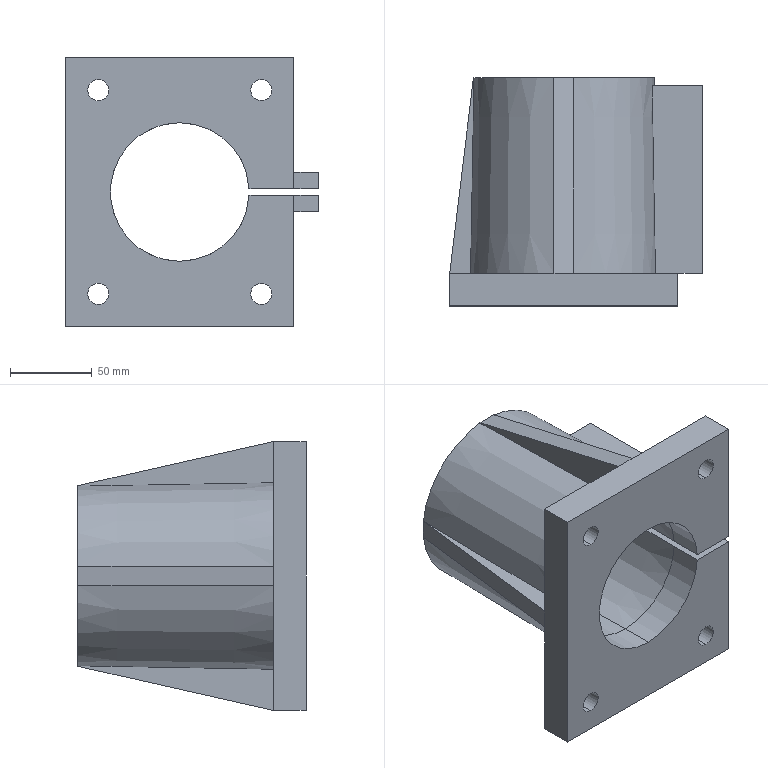Part | STEP file | csb-00004 | 1 solid | 48 faces | box 155 x 140 x 165 mm | volume 928209 mm3 | plane 30 | cylinder 11 | cone 7 | commonest cylinder face diameters 13 x8 85 x3
STEP:
#1=CARTESIAN_POINT('',(0.,20.,-42.5));
#2=VERTEX_POINT('',#1);
#3=CARTESIAN_POINT('',(0.,20.,42.5));
#4=VERTEX_POINT('',#3);
#5=CARTESIAN_POINT('',(0.,20.,0.));
#6=DIRECTION('',(0.,1.,0.));
#7=DIRECTION('',(0.,0.,1.));
#8=AXIS2_PLACEMENT_3D('',#5,#6,#7);
#9=CIRCLE('',#8,42.5);
#10=EDGE_CURVE('',#2,#4,#9,.T.);
#11=ORIENTED_EDGE('',*,*,#10,.F.);
#12=CARTESIAN_POINT('',(0.,140.,-44.595));
#13=VERTEX_POINT('',#12);
#14=CARTESIAN_POINT('',(0.,20.,-42.5));
#15=DIRECTION('',(0.,0.9998,-0.01745));
#16=VECTOR('',#15,1000.);
#17=LINE('',#14,#16);
#18=EDGE_CURVE('',#2,#13,#17,.T.);
#19=ORIENTED_EDGE('',*,*,#18,.T.);
#20=CARTESIAN_POINT('',(0.,140.,44.595));
#21=VERTEX_POINT('',#20);
#22=CARTESIAN_POINT('',(0.,140.,0.));
#23=DIRECTION('',(0.,1.,0.));
#24=DIRECTION('',(0.,0.,1.));
#25=AXIS2_PLACEMENT_3D('',#22,#23,#24);
#26=CIRCLE('',#25,44.595);
#27=EDGE_CURVE('',#13,#21,#26,.T.);
#28=ORIENTED_EDGE('',*,*,#27,.T.);
#29=CARTESIAN_POINT('',(0.,20.,42.5));
#30=DIRECTION('',(0.,0.9998,0.01745));
#31=VECTOR('',#30,1000.);
#32=LINE('',#29,#31);
#33=EDGE_CURVE('',#4,#21,#32,.T.);
#34=ORIENTED_EDGE('',*,*,#33,.F.);
#35=EDGE_LOOP('',(#11,#19,#28,#34));
#36=FACE_OUTER_BOUND('',#35,.T.);
#37=CARTESIAN_POINT('',(0.,20.,0.));
#38=DIRECTION('',(0.,1.,0.));
#39=DIRECTION('',(0.,0.,1.));
#40=AXIS2_PLACEMENT_3D('',#37,#38,#39);
#41=CONICAL_SURFACE('',#40,42.5,0.01745);
#42=ADVANCED_FACE('',(#36),#41,.F.);
#43=CARTESIAN_POINT('',(42.453,20.,2.));
#44=VERTEX_POINT('',#43);
#45=CARTESIAN_POINT('',(0.,20.,0.));
#46=DIRECTION('',(0.,1.,0.));
#47=DIRECTION('',(0.,0.,1.));
#48=AXIS2_PLACEMENT_3D('',#45,#46,#47);
#49=CIRCLE('',#48,42.5);
#50=EDGE_CURVE('',#4,#44,#49,.T.);
#51=ORIENTED_EDGE('',*,*,#50,.F.);
#52=ORIENTED_EDGE('',*,*,#33,.T.);
#53=CARTESIAN_POINT('',(44.55,140.,2.));
#54=VERTEX_POINT('',#53);
#55=CARTESIAN_POINT('',(0.,140.,0.));
#56=DIRECTION('',(0.,1.,0.));
#57=DIRECTION('',(0.,0.,1.));
#58=AXIS2_PLACEMENT_3D('',#55,#56,#57);
#59=CIRCLE('',#58,44.595);
#60=EDGE_CURVE('',#21,#54,#59,.T.);
#61=ORIENTED_EDGE('',*,*,#60,.T.);
#62=CARTESIAN_POINT('',(42.453,20.,2.));
#63=CARTESIAN_POINT('',(42.539,24.954,2.));
#64=CARTESIAN_POINT('',(42.626,29.908,2.));
#65=CARTESIAN_POINT('',(42.713,34.862,2.));
#66=CARTESIAN_POINT('',(43.202,62.875,2.));
#67=CARTESIAN_POINT('',(43.692,90.888,2.));
#68=CARTESIAN_POINT('',(44.181,118.901,2.));
#69=CARTESIAN_POINT('',(44.304,125.934,2.));
#70=CARTESIAN_POINT('',(44.427,132.967,2.));
#71=CARTESIAN_POINT('',(44.55,140.,2.));
#72=B_SPLINE_CURVE_WITH_KNOTS('',3,(#62,#63,#64,#65,#66,#67,#68,#69,#70,#71),.UNSPECIFIED.,.F.,.F.,(4,3,3,4),(0.06919,0.08405,0.1681,0.1892),.UNSPECIFIED.);
#73=EDGE_CURVE('',#44,#54,#72,.T.);
#74=ORIENTED_EDGE('',*,*,#73,.F.);
#75=EDGE_LOOP('',(#51,#52,#61,#74));
#76=FACE_OUTER_BOUND('',#75,.T.);
#77=CARTESIAN_POINT('',(0.,20.,0.));
#78=DIRECTION('',(0.,1.,0.));
#79=DIRECTION('',(0.,0.,1.));
#80=AXIS2_PLACEMENT_3D('',#77,#78,#79);
#81=CONICAL_SURFACE('',#80,42.5,0.01745);
#82=ADVANCED_FACE('',(#76),#81,.F.);
#83=CARTESIAN_POINT('',(50.,20.,-69.));
#84=VERTEX_POINT('',#83);
#85=CARTESIAN_POINT('',(50.,20.,-56.));
#86=VERTEX_POINT('',#85);
#87=CARTESIAN_POINT('',(50.,20.,-62.5));
#88=DIRECTION('',(0.,1.,0.));
#89=DIRECTION('',(0.,0.,1.));
#90=AXIS2_PLACEMENT_3D('',#87,#88,#89);
#91=CIRCLE('',#90,6.5);
#92=EDGE_CURVE('',#84,#86,#91,.T.);
#93=ORIENTED_EDGE('',*,*,#92,.T.);
#94=CARTESIAN_POINT('',(50.,0.,-56.));
#95=VERTEX_POINT('',#94);
#96=CARTESIAN_POINT('',(50.,20.,-56.));
#97=DIRECTION('',(0.,-1.,0.));
#98=VECTOR('',#97,1000.);
#99=LINE('',#96,#98);
#100=EDGE_CURVE('',#86,#95,#99,.T.);
#101=ORIENTED_EDGE('',*,*,#100,.T.);
#102=CARTESIAN_POINT('',(50.,0.,-69.));
#103=VERTEX_POINT('',#102);
#104=CARTESIAN_POINT('',(50.,0.,-62.5));
#105=DIRECTION('',(0.,1.,0.));
#106=DIRECTION('',(0.,0.,1.));
#107=AXIS2_PLACEMENT_3D('',#104,#105,#106);
#108=CIRCLE('',#107,6.5);
#109=EDGE_CURVE('',#103,#95,#108,.T.);
#110=ORIENTED_EDGE('',*,*,#109,.F.);
#111=CARTESIAN_POINT('',(50.,20.,-69.));
#112=DIRECTION('',(0.,-1.,0.));
#113=VECTOR('',#112,1000.);
#114=LINE('',#111,#113);
#115=EDGE_CURVE('',#84,#103,#114,.T.);
#116=ORIENTED_EDGE('',*,*,#115,.F.);
#117=EDGE_LOOP('',(#93,#101,#110,#116));
#118=FACE_OUTER_BOUND('',#117,.T.);
#119=CARTESIAN_POINT('',(50.,20.,-62.5));
#120=DIRECTION('',(0.,-1.,0.));
#121=DIRECTION('',(0.,0.,-1.));
#122=AXIS2_PLACEMENT_3D('',#119,#120,#121);
#123=CYLINDRICAL_SURFACE('',#122,6.5);
#124=ADVANCED_FACE('',(#118),#123,.F.);
#125=CARTESIAN_POINT('',(50.,20.,56.));
#126=VERTEX_POINT('',#125);
#127=CARTESIAN_POINT('',(50.,20.,69.));
#128=VERTEX_POINT('',#127);
#129=CARTESIAN_POINT('',(50.,20.,62.5));
#130=DIRECTION('',(0.,1.,0.));
#131=DIRECTION('',(0.,0.,1.));
#132=AXIS2_PLACEMENT_3D('',#129,#130,#131);
#133=CIRCLE('',#132,6.5);
#134=EDGE_CURVE('',#126,#128,#133,.T.);
#135=ORIENTED_EDGE('',*,*,#134,.T.);
#136=CARTESIAN_POINT('',(50.,0.,69.));
#137=VERTEX_POINT('',#136);
#138=CARTESIAN_POINT('',(50.,20.,69.));
#139=DIRECTION('',(0.,-1.,0.));
#140=VECTOR('',#139,1000.);
#141=LINE('',#138,#140);
#142=EDGE_CURVE('',#128,#137,#141,.T.);
#143=ORIENTED_EDGE('',*,*,#142,.T.);
#144=CARTESIAN_POINT('',(50.,0.,56.));
#145=VERTEX_POINT('',#144);
#146=CARTESIAN_POINT('',(50.,0.,62.5));
#147=DIRECTION('',(0.,1.,0.));
#148=DIRECTION('',(0.,0.,1.));
#149=AXIS2_PLACEMENT_3D('',#146,#147,#148);
#150=CIRCLE('',#149,6.5);
#151=EDGE_CURVE('',#145,#137,#150,.T.);
#152=ORIENTED_EDGE('',*,*,#151,.F.);
#153=CARTESIAN_POINT('',(50.,20.,56.));
#154=DIRECTION('',(0.,-1.,0.));
#155=VECTOR('',#154,1000.);
#156=LINE('',#153,#155);
#157=EDGE_CURVE('',#126,#145,#156,.T.);
#158=ORIENTED_EDGE('',*,*,#157,.F.);
#159=EDGE_LOOP('',(#135,#143,#152,#158));
#160=FACE_OUTER_BOUND('',#159,.T.);
#161=CARTESIAN_POINT('',(50.,20.,62.5));
#162=DIRECTION('',(0.,-1.,0.));
#163=DIRECTION('',(0.,0.,-1.));
#164=AXIS2_PLACEMENT_3D('',#161,#162,#163);
#165=CYLINDRICAL_SURFACE('',#164,6.5);
#166=ADVANCED_FACE('',(#160),#165,.F.);
#167=CARTESIAN_POINT('',(-50.,20.,56.));
#168=VERTEX_POINT('',#167);
#169=CARTESIAN_POINT('',(-50.,20.,69.));
#170=VERTEX_POINT('',#169);
#171=CARTESIAN_POINT('',(-50.,20.,62.5));
#172=DIRECTION('',(0.,1.,0.));
#173=DIRECTION('',(0.,0.,1.));
#174=AXIS2_PLACEMENT_3D('',#171,#172,#173);
#175=CIRCLE('',#174,6.5);
#176=EDGE_CURVE('',#168,#170,#175,.T.);
#177=ORIENTED_EDGE('',*,*,#176,.T.);
#178=CARTESIAN_POINT('',(-50.,0.,69.));
#179=VERTEX_POINT('',#178);
#180=CARTESIAN_POINT('',(-50.,20.,69.));
#181=DIRECTION('',(0.,-1.,0.));
#182=VECTOR('',#181,1000.);
#183=LINE('',#180,#182);
#184=EDGE_CURVE('',#170,#179,#183,.T.);
#185=ORIENTED_EDGE('',*,*,#184,.T.);
#186=CARTESIAN_POINT('',(-50.,0.,56.));
#187=VERTEX_POINT('',#186);
#188=CARTESIAN_POINT('',(-50.,0.,62.5));
#189=DIRECTION('',(0.,1.,0.));
#190=DIRECTION('',(0.,0.,1.));
#191=AXIS2_PLACEMENT_3D('',#188,#189,#190);
#192=CIRCLE('',#191,6.5);
#193=EDGE_CURVE('',#187,#179,#192,.T.);
#194=ORIENTED_EDGE('',*,*,#193,.F.);
#195=CARTESIAN_POINT('',(-50.,20.,56.));
#196=DIRECTION('',(0.,-1.,0.));
#197=VECTOR('',#196,1000.);
#198=LINE('',#195,#197);
#199=EDGE_CURVE('',#168,#187,#198,.T.);
#200=ORIENTED_EDGE('',*,*,#199,.F.);
#201=EDGE_LOOP('',(#177,#185,#194,#200));
#202=FACE_OUTER_BOUND('',#201,.T.);
#203=CARTESIAN_POINT('',(-50.,20.,62.5));
#204=DIRECTION('',(0.,-1.,0.));
#205=DIRECTION('',(0.,0.,-1.));
#206=AXIS2_PLACEMENT_3D('',#203,#204,#205);
#207=CYLINDRICAL_SURFACE('',#206,6.5);
#208=ADVANCED_FACE('',(#202),#207,.F.);
#209=CARTESIAN_POINT('',(-50.,20.,-69.));
#210=VERTEX_POINT('',#209);
#211=CARTESIAN_POINT('',(-50.,20.,-56.));
#212=VERTEX_POINT('',#211);
#213=CARTESIAN_POINT('',(-50.,20.,-62.5));
#214=DIRECTION('',(0.,1.,0.));
#215=DIRECTION('',(0.,0.,1.));
#216=AXIS2_PLACEMENT_3D('',#213,#214,#215);
#217=CIRCLE('',#216,6.5);
#218=EDGE_CURVE('',#210,#212,#217,.T.);
#219=ORIENTED_EDGE('',*,*,#218,.T.);
#220=CARTESIAN_POINT('',(-50.,0.,-56.));
#221=VERTEX_POINT('',#220);
#222=CARTESIAN_POINT('',(-50.,20.,-56.));
#223=DIRECTION('',(0.,-1.,0.));
#224=VECTOR('',#223,1000.);
#225=LINE('',#222,#224);
#226=EDGE_CURVE('',#212,#221,#225,.T.);
#227=ORIENTED_EDGE('',*,*,#226,.T.);
#228=CARTESIAN_POINT('',(-50.,0.,-69.));
#229=VERTEX_POINT('',#228);
#230=CARTESIAN_POINT('',(-50.,0.,-62.5));
#231=DIRECTION('',(0.,1.,0.));
#232=DIRECTION('',(0.,0.,1.));
#233=AXIS2_PLACEMENT_3D('',#230,#231,#232);
#234=CIRCLE('',#233,6.5);
#235=EDGE_CURVE('',#229,#221,#234,.T.);
#236=ORIENTED_EDGE('',*,*,#235,.F.);
#237=CARTESIAN_POINT('',(-50.,20.,-69.));
#238=DIRECTION('',(0.,-1.,0.));
#239=VECTOR('',#238,1000.);
#240=LINE('',#237,#239);
#241=EDGE_CURVE('',#210,#229,#240,.T.);
#242=ORIENTED_EDGE('',*,*,#241,.F.);
#243=EDGE_LOOP('',(#219,#227,#236,#242));
#244=FACE_OUTER_BOUND('',#243,.T.);
#245=CARTESIAN_POINT('',(-50.,20.,-62.5));
#246=DIRECTION('',(0.,-1.,0.));
#247=DIRECTION('',(0.,0.,-1.));
#248=AXIS2_PLACEMENT_3D('',#245,#246,#247);
#249=CYLINDRICAL_SURFACE('',#248,6.5);
#250=ADVANCED_FACE('',(#244),#249,.F.);
#251=ORIENTED_EDGE('',*,*,#10,.T.);
#252=CARTESIAN_POINT('',(0.,0.,42.5));
#253=VERTEX_POINT('',#252);
#254=CARTESIAN_POINT('',(0.,20.,42.5));
#255=DIRECTION('',(0.,-1.,0.));
#256=VECTOR('',#255,1000.);
#257=LINE('',#254,#256);
#258=EDGE_CURVE('',#4,#253,#257,.T.);
#259=ORIENTED_EDGE('',*,*,#258,.T.);
#260=CARTESIAN_POINT('',(0.,0.,-42.5));
#261=VERTEX_POINT('',#260);
#262=CARTESIAN_POINT('',(0.,0.,0.));
#263=DIRECTION('',(0.,1.,0.));
#264=DIRECTION('',(0.,0.,1.));
#265=AXIS2_PLACEMENT_3D('',#262,#263,#264);
#266=CIRCLE('',#265,42.5);
#267=EDGE_CURVE('',#261,#253,#266,.T.);
#268=ORIENTED_EDGE('',*,*,#267,.F.);
#269=CARTESIAN_POINT('',(0.,20.,-42.5));
#270=DIRECTION('',(0.,-1.,0.));
#271=VECTOR('',#270,1000.);
#272=LINE('',#269,#271);
#273=EDGE_CURVE('',#2,#261,#272,.T.);
#274=ORIENTED_EDGE('',*,*,#273,.F.);
#275=EDGE_LOOP('',(#251,#259,#268,#274));
#276=FACE_OUTER_BOUND('',#275,.T.);
#277=CARTESIAN_POINT('',(0.,20.,0.));
#278=DIRECTION('',(0.,-1.,0.));
#279=DIRECTION('',(0.,0.,-1.));
#280=AXIS2_PLACEMENT_3D('',#277,#278,#279);
#281=CYLINDRICAL_SURFACE('',#280,42.5);
#282=ADVANCED_FACE('',(#276),#281,.F.);
#283=CARTESIAN_POINT('',(42.453,20.,-2.));
#284=VERTEX_POINT('',#283);
#285=CARTESIAN_POINT('',(0.,20.,0.));
#286=DIRECTION('',(0.,1.,0.));
#287=DIRECTION('',(0.,0.,1.));
#288=AXIS2_PLACEMENT_3D('',#285,#286,#287);
#289=CIRCLE('',#288,42.5);
#290=EDGE_CURVE('',#284,#2,#289,.T.);
#291=ORIENTED_EDGE('',*,*,#290,.T.);
#292=ORIENTED_EDGE('',*,*,#273,.T.);
#293=CARTESIAN_POINT('',(42.453,0.,-2.));
#294=VERTEX_POINT('',#293);
#295=CARTESIAN_POINT('',(0.,0.,0.));
#296=DIRECTION('',(0.,1.,0.));
#297=DIRECTION('',(0.,0.,1.));
#298=AXIS2_PLACEMENT_3D('',#295,#296,#297);
#299=CIRCLE('',#298,42.5);
#300=EDGE_CURVE('',#294,#261,#299,.T.);
#301=ORIENTED_EDGE('',*,*,#300,.F.);
#302=CARTESIAN_POINT('',(42.453,20.,-2.));
#303=DIRECTION('',(0.,-1.,0.));
#304=VECTOR('',#303,1000.);
#305=LINE('',#302,#304);
#306=EDGE_CURVE('',#284,#294,#305,.T.);
#307=ORIENTED_EDGE('',*,*,#306,.F.);
#308=EDGE_LOOP('',(#291,#292,#301,#307));
#309=FACE_OUTER_BOUND('',#308,.T.);
#310=CARTESIAN_POINT('',(0.,20.,0.));
#311=DIRECTION('',(0.,-1.,0.));
#312=DIRECTION('',(0.,0.,-1.));
#313=AXIS2_PLACEMENT_3D('',#310,#311,#312);
#314=CYLINDRICAL_SURFACE('',#313,42.5);
#315=ADVANCED_FACE('',(#309),#314,.F.);
#316=CARTESIAN_POINT('',(54.18,135.,12.));
#317=VERTEX_POINT('',#316);
#318=CARTESIAN_POINT('',(55.457,135.,2.));
#319=VERTEX_POINT('',#318);
#320=CARTESIAN_POINT('',(0.,135.,0.));
#321=DIRECTION('',(0.,1.,0.));
#322=DIRECTION('',(0.,0.,1.));
#323=AXIS2_PLACEMENT_3D('',#320,#321,#322);
#324=CIRCLE('',#323,55.493);
#325=EDGE_CURVE('',#317,#319,#324,.T.);
#326=ORIENTED_EDGE('',*,*,#325,.T.);
#327=CARTESIAN_POINT('',(55.369,140.,2.));
#328=VERTEX_POINT('',#327);
#329=CARTESIAN_POINT('',(55.457,135.,2.));
#330=CARTESIAN_POINT('',(55.428,136.667,2.));
#331=CARTESIAN_POINT('',(55.398,138.333,2.));
#332=CARTESIAN_POINT('',(55.369,140.,2.));
#333=B_SPLINE_CURVE_WITH_KNOTS('',3,(#329,#330,#331,#332),.UNSPECIFIED.,.F.,.F.,(4,4),(0.3856,0.3906),.UNSPECIFIED.);
#334=EDGE_CURVE('',#319,#328,#333,.T.);
#335=ORIENTED_EDGE('',*,*,#334,.T.);
#336=CARTESIAN_POINT('',(6.,140.,55.08));
#337=VERTEX_POINT('',#336);
#338=CARTESIAN_POINT('',(0.,140.,0.));
#339=DIRECTION('',(0.,1.,0.));
#340=DIRECTION('',(0.,0.,1.));
#341=AXIS2_PLACEMENT_3D('',#338,#339,#340);
#342=CIRCLE('',#341,55.405);
#343=EDGE_CURVE('',#337,#328,#342,.T.);
#344=ORIENTED_EDGE('',*,*,#343,.F.);
#345=CARTESIAN_POINT('',(6.,20.,57.186));
#346=VERTEX_POINT('',#345);
#347=CARTESIAN_POINT('',(6.,140.,55.08));
#348=CARTESIAN_POINT('',(6.,105.015,55.694));
#349=CARTESIAN_POINT('',(6.,70.029,56.308));
#350=CARTESIAN_POINT('',(6.,35.044,56.922));
#351=CARTESIAN_POINT('',(6.,30.029,57.01));
#352=CARTESIAN_POINT('',(6.,25.015,57.098));
#353=CARTESIAN_POINT('',(6.,20.,57.186));
#354=B_SPLINE_CURVE_WITH_KNOTS('',3,(#347,#348,#349,#350,#351,#352,#353),.UNSPECIFIED.,.F.,.F.,(4,3,4),(0.2243,0.3293,0.3443),.UNSPECIFIED.);
#355=EDGE_CURVE('',#337,#346,#354,.T.);
#356=ORIENTED_EDGE('',*,*,#355,.T.);
#357=CARTESIAN_POINT('',(56.234,20.,12.));
#358=VERTEX_POINT('',#357);
#359=CARTESIAN_POINT('',(0.,20.,0.));
#360=DIRECTION('',(0.,1.,0.));
#361=DIRECTION('',(0.,0.,-1.));
#362=AXIS2_PLACEMENT_3D('',#359,#360,#361);
#363=CIRCLE('',#362,57.5);
#364=EDGE_CURVE('',#346,#358,#363,.T.);
#365=ORIENTED_EDGE('',*,*,#364,.T.);
#366=CARTESIAN_POINT('',(54.18,135.,12.));
#367=CARTESIAN_POINT('',(54.779,101.487,12.));
#368=CARTESIAN_POINT('',(55.378,67.973,12.));
#369=CARTESIAN_POINT('',(55.976,34.46,12.));
#370=CARTESIAN_POINT('',(56.062,29.64,12.));
#371=CARTESIAN_POINT('',(56.148,24.82,12.));
#372=CARTESIAN_POINT('',(56.234,20.,12.));
#373=B_SPLINE_CURVE_WITH_KNOTS('',3,(#366,#367,#368,#369,#370,#371,#372),.UNSPECIFIED.,.F.,.F.,(4,3,4),(0.2223,0.3229,0.3374),.UNSPECIFIED.);
#374=EDGE_CURVE('',#317,#358,#373,.T.);
#375=ORIENTED_EDGE('',*,*,#374,.F.);
#376=EDGE_LOOP('',(#326,#335,#344,#356,#365,#375));
#377=FACE_OUTER_BOUND('',#376,.T.);
#378=CARTESIAN_POINT('',(0.,20.,0.));
#379=DIRECTION('',(0.,-1.,0.));
#380=DIRECTION('',(0.,0.,1.));
#381=AXIS2_PLACEMENT_3D('',#378,#379,#380);
#382=CONICAL_SURFACE('',#381,57.5,0.01745);
#383=ADVANCED_FACE('',(#377),#382,.T.);
#384=CARTESIAN_POINT('',(70.,0.,82.5));
#385=VERTEX_POINT('',#384);
#386=CARTESIAN_POINT('',(70.,0.,2.));
#387=VERTEX_POINT('',#386);
#388=CARTESIAN_POINT('',(70.,0.,82.5));
#389=DIRECTION('',(0.,0.,-1.));
#390=VECTOR('',#389,1000.);
#391=LINE('',#388,#390);
#392=EDGE_CURVE('',#385,#387,#391,.T.);
#393=ORIENTED_EDGE('',*,*,#392,.T.);
#394=CARTESIAN_POINT('',(70.,20.,2.));
#395=VERTEX_POINT('',#394);
#396=CARTESIAN_POINT('',(70.,20.,2.));
#397=DIRECTION('',(0.,1.,0.));
#398=VECTOR('',#397,1000.);
#399=LINE('',#396,#398);
#400=EDGE_CURVE('',#387,#395,#399,.T.);
#401=ORIENTED_EDGE('',*,*,#400,.T.);
#402=CARTESIAN_POINT('',(70.,20.,12.));
#403=VERTEX_POINT('',#402);
#404=CARTESIAN_POINT('',(70.,20.,82.5));
#405=DIRECTION('',(0.,0.,-1.));
#406=VECTOR('',#405,1000.);
#407=LINE('',#404,#406);
#408=EDGE_CURVE('',#403,#395,#407,.T.);
#409=ORIENTED_EDGE('',*,*,#408,.F.);
#410=CARTESIAN_POINT('',(70.,20.,82.5));
#411=VERTEX_POINT('',#410);
#412=CARTESIAN_POINT('',(70.,20.,82.5));
#413=DIRECTION('',(0.,0.,-1.));
#414=VECTOR('',#413,1000.);
#415=LINE('',#412,#414);
#416=EDGE_CURVE('',#411,#403,#415,.T.);
#417=ORIENTED_EDGE('',*,*,#416,.F.);
#418=CARTESIAN_POINT('',(70.,20.,82.5));
#419=DIRECTION('',(0.,-1.,0.));
#420=VECTOR('',#419,1000.);
#421=LINE('',#418,#420);
#422=EDGE_CURVE('',#411,#385,#421,.T.);
#423=ORIENTED_EDGE('',*,*,#422,.T.);
#424=EDGE_LOOP('',(#393,#401,#409,#417,#423));
#425=FACE_OUTER_BOUND('',#424,.T.);
#426=CARTESIAN_POINT('',(70.,20.,82.5));
#427=DIRECTION('',(-1.,0.,0.));
#428=DIRECTION('',(0.,0.,1.));
#429=AXIS2_PLACEMENT_3D('',#426,#427,#428);
#430=PLANE('',#429);
#431=ADVANCED_FACE('',(#425),#430,.F.);
#432=CARTESIAN_POINT('',(85.,135.,2.));
#433=VERTEX_POINT('',#432);
#434=CARTESIAN_POINT('',(45.,135.,2.));
#435=DIRECTION('',(1.,0.,0.));
#436=VECTOR('',#435,1000.);
#437=LINE('',#434,#436);
#438=EDGE_CURVE('',#319,#433,#437,.T.);
#439=ORIENTED_EDGE('',*,*,#438,.F.);
#440=ORIENTED_EDGE('',*,*,#325,.F.);
#441=CARTESIAN_POINT('',(85.,135.,12.));
#442=VERTEX_POINT('',#441);
#443=CARTESIAN_POINT('',(45.,135.,12.));
#444=DIRECTION('',(-1.,0.,0.));
#445=VECTOR('',#444,1000.);
#446=LINE('',#443,#445);
#447=EDGE_CURVE('',#442,#317,#446,.T.);
#448=ORIENTED_EDGE('',*,*,#447,.F.);
#449=CARTESIAN_POINT('',(85.,135.,-12.));
#450=DIRECTION('',(0.,0.,1.));
#451=VECTOR('',#450,1000.);
#452=LINE('',#449,#451);
#453=EDGE_CURVE('',#433,#442,#452,.T.);
#454=ORIENTED_EDGE('',*,*,#453,.F.);
#455=EDGE_LOOP('',(#439,#440,#448,#454));
#456=FACE_OUTER_BOUND('',#455,.T.);
#457=CARTESIAN_POINT('',(45.,135.,-12.));
#458=DIRECTION('',(0.,1.,0.));
#459=DIRECTION('',(0.,0.,1.));
#460=AXIS2_PLACEMENT_3D('',#457,#458,#459);
#461=PLANE('',#460);
#462=ADVANCED_FACE('',(#456),#461,.T.);
#463=CARTESIAN_POINT('',(85.,20.,2.));
#464=VERTEX_POINT('',#463);
#465=CARTESIAN_POINT('',(85.,20.,2.));
#466=DIRECTION('',(-1.,0.,0.));
#467=VECTOR('',#466,1000.);
#468=LINE('',#465,#467);
#469=EDGE_CURVE('',#464,#395,#468,.T.);
#470=ORIENTED_EDGE('',*,*,#469,.F.);
#471=CARTESIAN_POINT('',(85.,20.,12.));
#472=VERTEX_POINT('',#471);
#473=CARTESIAN_POINT('',(85.,20.,-12.));
#474=DIRECTION('',(0.,0.,1.));
#475=VECTOR('',#474,1000.);
#476=LINE('',#473,#475);
#477=EDGE_CURVE('',#464,#472,#476,.T.);
#478=ORIENTED_EDGE('',*,*,#477,.T.);
#479=CARTESIAN_POINT('',(85.,20.,12.));
#480=DIRECTION('',(1.,0.,0.));
#481=VECTOR('',#480,1000.);
#482=LINE('',#479,#481);
#483=EDGE_CURVE('',#403,#472,#482,.T.);
#484=ORIENTED_EDGE('',*,*,#483,.F.);
#485=ORIENTED_EDGE('',*,*,#408,.T.);
#486=EDGE_LOOP('',(#470,#478,#484,#485));
#487=FACE_OUTER_BOUND('',#486,.T.);
#488=CARTESIAN_POINT('',(85.,20.,-12.));
#489=DIRECTION('',(0.,-1.,0.));
#490=DIRECTION('',(1.,0.,0.));
#491=AXIS2_PLACEMENT_3D('',#488,#489,#490);
#492=PLANE('',#491);
#493=ADVANCED_FACE('',(#487),#492,.T.);
#494=CARTESIAN_POINT('',(85.,135.,2.));
#495=DIRECTION('',(0.,-1.,0.));
#496=VECTOR('',#495,1000.);
#497=LINE('',#494,#496);
#498=EDGE_CURVE('',#433,#464,#497,.T.);
#499=ORIENTED_EDGE('',*,*,#498,.F.);
#500=ORIENTED_EDGE('',*,*,#453,.T.);
#501=CARTESIAN_POINT('',(85.,135.,12.));
#502=DIRECTION('',(0.,1.,0.));
#503=VECTOR('',#502,1000.);
#504=LINE('',#501,#503);
#505=EDGE_CURVE('',#472,#442,#504,.T.);
#506=ORIENTED_EDGE('',*,*,#505,.F.);
#507=ORIENTED_EDGE('',*,*,#477,.F.);
#508=EDGE_LOOP('',(#499,#500,#506,#507));
#509=FACE_OUTER_BOUND('',#508,.T.);
#510=CARTESIAN_POINT('',(85.,135.,-12.));
#511=DIRECTION('',(1.,0.,0.));
#512=DIRECTION('',(0.,1.,0.));
#513=AXIS2_PLACEMENT_3D('',#510,#511,#512);
#514=PLANE('',#513);
#515=ADVANCED_FACE('',(#509),#514,.T.);
#516=ORIENTED_EDGE('',*,*,#134,.F.);
#517=CARTESIAN_POINT('',(50.,20.,62.5));
#518=DIRECTION('',(0.,1.,0.));
#519=DIRECTION('',(0.,0.,1.));
#520=AXIS2_PLACEMENT_3D('',#517,#518,#519);
#521=CIRCLE('',#520,6.5);
#522=EDGE_CURVE('',#128,#126,#521,.T.);
#523=ORIENTED_EDGE('',*,*,#522,.F.);
#524=EDGE_LOOP('',(#516,#523));
#525=FACE_BOUND('',#524,.T.);
#526=CARTESIAN_POINT('',(85.,20.,12.));
#527=DIRECTION('',(1.,0.,0.));
#528=VECTOR('',#527,1000.);
#529=LINE('',#526,#528);
#530=EDGE_CURVE('',#358,#403,#529,.T.);
#531=ORIENTED_EDGE('',*,*,#530,.F.);
#532=ORIENTED_EDGE('',*,*,#364,.F.);
#533=CARTESIAN_POINT('',(6.,20.,82.5));
#534=VERTEX_POINT('',#533);
#535=CARTESIAN_POINT('',(6.,20.,82.5));
#536=DIRECTION('',(0.,0.,-1.));
#537=VECTOR('',#536,1000.);
#538=LINE('',#535,#537);
#539=EDGE_CURVE('',#534,#346,#538,.T.);
#540=ORIENTED_EDGE('',*,*,#539,.F.);
#541=CARTESIAN_POINT('',(-70.,20.,82.5));
#542=DIRECTION('',(1.,0.,0.));
#543=VECTOR('',#542,1000.);
#544=LINE('',#541,#543);
#545=EDGE_CURVE('',#534,#411,#544,.T.);
#546=ORIENTED_EDGE('',*,*,#545,.T.);
#547=ORIENTED_EDGE('',*,*,#416,.T.);
#548=EDGE_LOOP('',(#531,#532,#540,#546,#547));
#549=FACE_OUTER_BOUND('',#548,.T.);
#550=CARTESIAN_POINT('',(-70.,20.,-82.5));
#551=DIRECTION('',(0.,-1.,0.));
#552=DIRECTION('',(0.,0.,-1.));
#553=AXIS2_PLACEMENT_3D('',#550,#551,#552);
#554=PLANE('',#553);
#555=ADVANCED_FACE('',(#525,#549),#554,.F.);
#556=ORIENTED_EDGE('',*,*,#218,.F.);
#557=CARTESIAN_POINT('',(-50.,20.,-62.5));
#558=DIRECTION('',(0.,1.,0.));
#559=DIRECTION('',(0.,0.,1.));
#560=AXIS2_PLACEMENT_3D('',#557,#558,#559);
#561=CIRCLE('',#560,6.5);
#562=EDGE_CURVE('',#212,#210,#561,.T.);
#563=ORIENTED_EDGE('',*,*,#562,.F.);
#564=EDGE_LOOP('',(#556,#563));
#565=FACE_BOUND('',#564,.T.);
#566=CARTESIAN_POINT('',(-70.,20.,-6.));
#567=VERTEX_POINT('',#566);
#568=CARTESIAN_POINT('',(-57.186,20.,-6.));
#569=VERTEX_POINT('',#568);
#570=CARTESIAN_POINT('',(-70.,20.,-6.));
#571=DIRECTION('',(1.,0.,0.));
#572=VECTOR('',#571,1000.);
#573=LINE('',#570,#572);
#574=EDGE_CURVE('',#567,#569,#573,.T.);
#575=ORIENTED_EDGE('',*,*,#574,.T.);
#576=CARTESIAN_POINT('',(-6.,20.,-57.186));
#577=VERTEX_POINT('',#576);
#578=CARTESIAN_POINT('',(0.,20.,0.));
#579=DIRECTION('',(0.,1.,0.));
#580=DIRECTION('',(0.,0.,-1.));
#581=AXIS2_PLACEMENT_3D('',#578,#579,#580);
#582=CIRCLE('',#581,57.5);
#583=EDGE_CURVE('',#577,#569,#582,.T.);
#584=ORIENTED_EDGE('',*,*,#583,.F.);
#585=CARTESIAN_POINT('',(-6.,20.,-82.5));
#586=VERTEX_POINT('',#585);
#587=CARTESIAN_POINT('',(-6.,20.,-82.5));
#588=DIRECTION('',(0.,0.,-1.));
#589=VECTOR('',#588,1000.);
#590=LINE('',#587,#589);
#591=EDGE_CURVE('',#577,#586,#590,.T.);
#592=ORIENTED_EDGE('',*,*,#591,.T.);
#593=CARTESIAN_POINT('',(-70.,20.,-82.5));
#594=VERTEX_POINT('',#593);
#595=CARTESIAN_POINT('',(-70.,20.,-82.5));
#596=DIRECTION('',(-1.,0.,0.));
#597=VECTOR('',#596,1000.);
#598=LINE('',#595,#597);
#599=EDGE_CURVE('',#586,#594,#598,.T.);
#600=ORIENTED_EDGE('',*,*,#599,.T.);
#601=CARTESIAN_POINT('',(-70.,20.,82.5));
#602=DIRECTION('',(0.,0.,1.));
#603=VECTOR('',#602,1000.);
#604=LINE('',#601,#603);
#605=EDGE_CURVE('',#594,#567,#604,.T.);
#606=ORIENTED_EDGE('',*,*,#605,.T.);
#607=EDGE_LOOP('',(#575,#584,#592,#600,#606));
#608=FACE_OUTER_BOUND('',#607,.T.);
#609=CARTESIAN_POINT('',(-70.,20.,-82.5));
#610=DIRECTION('',(0.,-1.,0.));
#611=DIRECTION('',(0.,0.,-1.));
#612=AXIS2_PLACEMENT_3D('',#609,#610,#611);
#613=PLANE('',#612);
#614=ADVANCED_FACE('',(#565,#608),#613,.F.);
#615=CARTESIAN_POINT('',(-55.08,140.,-6.));
#616=VERTEX_POINT('',#615);
#617=CARTESIAN_POINT('',(-55.08,140.,-6.));
#618=CARTESIAN_POINT('',(-55.694,105.015,-6.));
#619=CARTESIAN_POINT('',(-56.308,70.03,-6.));
#620=CARTESIAN_POINT('',(-56.922,35.045,-6.));
#621=CARTESIAN_POINT('',(-57.01,30.03,-6.));
#622=CARTESIAN_POINT('',(-57.098,25.015,-6.));
#623=CARTESIAN_POINT('',(-57.186,20.,-6.));
#624=B_SPLINE_CURVE_WITH_KNOTS('',3,(#617,#618,#619,#620,#621,#622,#623),.UNSPECIFIED.,.F.,.F.,(4,3,4),(0.2244,0.3293,0.3444),.UNSPECIFIED.);
#625=EDGE_CURVE('',#616,#569,#624,.T.);
#626=ORIENTED_EDGE('',*,*,#625,.F.);
#627=CARTESIAN_POINT('',(-6.,140.,-55.08));
#628=VERTEX_POINT('',#627);
#629=CARTESIAN_POINT('',(0.,140.,0.));
#630=DIRECTION('',(0.,1.,0.));
#631=DIRECTION('',(0.,0.,1.));
#632=AXIS2_PLACEMENT_3D('',#629,#630,#631);
#633=CIRCLE('',#632,55.405);
#634=EDGE_CURVE('',#628,#616,#633,.T.);
#635=ORIENTED_EDGE('',*,*,#634,.F.);
#636=CARTESIAN_POINT('',(-6.,20.,-57.186));
#637=CARTESIAN_POINT('',(-6.,25.015,-57.098));
#638=CARTESIAN_POINT('',(-6.,30.029,-57.01));
#639=CARTESIAN_POINT('',(-6.,35.044,-56.922));
#640=CARTESIAN_POINT('',(-6.,70.029,-56.308));
#641=CARTESIAN_POINT('',(-6.,105.015,-55.694));
#642=CARTESIAN_POINT('',(-6.,140.,-55.08));
#643=B_SPLINE_CURVE_WITH_KNOTS('',3,(#636,#637,#638,#639,#640,#641,#642),.UNSPECIFIED.,.F.,.F.,(4,3,4),(0.09746,0.1125,0.2175),.UNSPECIFIED.);
#644=EDGE_CURVE('',#577,#628,#643,.T.);
#645=ORIENTED_EDGE('',*,*,#644,.F.);
#646=ORIENTED_EDGE('',*,*,#583,.T.);
#647=EDGE_LOOP('',(#626,#635,#645,#646));
#648=FACE_OUTER_BOUND('',#647,.T.);
#649=CARTESIAN_POINT('',(0.,20.,0.));
#650=DIRECTION('',(0.,-1.,0.));
#651=DIRECTION('',(0.,0.,1.));
#652=AXIS2_PLACEMENT_3D('',#649,#650,#651);
#653=CONICAL_SURFACE('',#652,57.5,0.01745);
#654=ADVANCED_FACE('',(#648),#653,.T.);
#655=ORIENTED_EDGE('',*,*,#176,.F.);
#656=CARTESIAN_POINT('',(-50.,20.,62.5));
#657=DIRECTION('',(0.,1.,0.));
#658=DIRECTION('',(0.,0.,1.));
#659=AXIS2_PLACEMENT_3D('',#656,#657,#658);
#660=CIRCLE('',#659,6.5);
#661=EDGE_CURVE('',#170,#168,#660,.T.);
#662=ORIENTED_EDGE('',*,*,#661,.F.);
#663=EDGE_LOOP('',(#655,#662));
#664=FACE_BOUND('',#663,.T.);
#665=CARTESIAN_POINT('',(-57.186,20.,6.));
#666=VERTEX_POINT('',#665);
#667=CARTESIAN_POINT('',(-6.,20.,57.186));
#668=VERTEX_POINT('',#667);
#669=CARTESIAN_POINT('',(0.,20.,0.));
#670=DIRECTION('',(0.,1.,0.));
#671=DIRECTION('',(0.,0.,-1.));
#672=AXIS2_PLACEMENT_3D('',#669,#670,#671);
#673=CIRCLE('',#672,57.5);
#674=EDGE_CURVE('',#666,#668,#673,.T.);
#675=ORIENTED_EDGE('',*,*,#674,.F.);
#676=CARTESIAN_POINT('',(-70.,20.,6.));
#677=VERTEX_POINT('',#676);
#678=CARTESIAN_POINT('',(-70.,20.,6.));
#679=DIRECTION('',(1.,0.,0.));
#680=VECTOR('',#679,1000.);
#681=LINE('',#678,#680);
#682=EDGE_CURVE('',#677,#666,#681,.T.);
#683=ORIENTED_EDGE('',*,*,#682,.F.);
#684=CARTESIAN_POINT('',(-70.,20.,82.5));
#685=VERTEX_POINT('',#684);
#686=CARTESIAN_POINT('',(-70.,20.,82.5));
#687=DIRECTION('',(0.,0.,1.));
#688=VECTOR('',#687,1000.);
#689=LINE('',#686,#688);
#690=EDGE_CURVE('',#677,#685,#689,.T.);
#691=ORIENTED_EDGE('',*,*,#690,.T.);
#692=CARTESIAN_POINT('',(-6.,20.,82.5));
#693=VERTEX_POINT('',#692);
#694=CARTESIAN_POINT('',(-70.,20.,82.5));
#695=DIRECTION('',(1.,0.,0.));
#696=VECTOR('',#695,1000.);
#697=LINE('',#694,#696);
#698=EDGE_CURVE('',#685,#693,#697,.T.);
#699=ORIENTED_EDGE('',*,*,#698,.T.);
#700=CARTESIAN_POINT('',(-6.,20.,82.5));
#701=DIRECTION('',(0.,0.,-1.));
#702=VECTOR('',#701,1000.);
#703=LINE('',#700,#702);
#704=EDGE_CURVE('',#693,#668,#703,.T.);
#705=ORIENTED_EDGE('',*,*,#704,.T.);
#706=EDGE_LOOP('',(#675,#683,#691,#699,#705));
#707=FACE_OUTER_BOUND('',#706,.T.);
#708=CARTESIAN_POINT('',(-70.,20.,-82.5));
#709=DIRECTION('',(0.,-1.,0.));
#710=DIRECTION('',(0.,0.,-1.));
#711=AXIS2_PLACEMENT_3D('',#708,#709,#710);
#712=PLANE('',#711);
#713=ADVANCED_FACE('',(#664,#707),#712,.F.);
#714=CARTESIAN_POINT('',(-55.08,140.,6.));
#715=VERTEX_POINT('',#714);
#716=CARTESIAN_POINT('',(-6.,140.,55.08));
#717=VERTEX_POINT('',#716);
#718=CARTESIAN_POINT('',(0.,140.,0.));
#719=DIRECTION('',(0.,1.,0.));
#720=DIRECTION('',(0.,0.,1.));
#721=AXIS2_PLACEMENT_3D('',#718,#719,#720);
#722=CIRCLE('',#721,55.405);
#723=EDGE_CURVE('',#715,#717,#722,.T.);
#724=ORIENTED_EDGE('',*,*,#723,.F.);
#725=CARTESIAN_POINT('',(-55.08,140.,6.));
#726=CARTESIAN_POINT('',(-55.694,105.015,6.));
#727=CARTESIAN_POINT('',(-56.308,70.03,6.));
#728=CARTESIAN_POINT('',(-56.922,35.045,6.));
#729=CARTESIAN_POINT('',(-57.01,30.03,6.));
#730=CARTESIAN_POINT('',(-57.098,25.015,6.));
#731=CARTESIAN_POINT('',(-57.186,20.,6.));
#732=B_SPLINE_CURVE_WITH_KNOTS('',3,(#725,#726,#727,#728,#729,#730,#731),.UNSPECIFIED.,.F.,.F.,(4,3,4),(0.2244,0.3293,0.3444),.UNSPECIFIED.);
#733=EDGE_CURVE('',#715,#666,#732,.T.);
#734=ORIENTED_EDGE('',*,*,#733,.T.);
#735=ORIENTED_EDGE('',*,*,#674,.T.);
#736=CARTESIAN_POINT('',(-6.,140.,55.08));
#737=CARTESIAN_POINT('',(-6.,105.015,55.694));
#738=CARTESIAN_POINT('',(-6.,70.029,56.308));
#739=CARTESIAN_POINT('',(-6.,35.044,56.922));
#740=CARTESIAN_POINT('',(-6.,30.029,57.01));
#741=CARTESIAN_POINT('',(-6.,25.015,57.098));
#742=CARTESIAN_POINT('',(-6.,20.,57.186));
#743=B_SPLINE_CURVE_WITH_KNOTS('',3,(#736,#737,#738,#739,#740,#741,#742),.UNSPECIFIED.,.F.,.F.,(4,3,4),(0.2243,0.3293,0.3443),.UNSPECIFIED.);
#744=EDGE_CURVE('',#717,#668,#743,.T.);
#745=ORIENTED_EDGE('',*,*,#744,.F.);
#746=EDGE_LOOP('',(#724,#734,#735,#745));
#747=FACE_OUTER_BOUND('',#746,.T.);
#748=CARTESIAN_POINT('',(0.,20.,0.));
#749=DIRECTION('',(0.,-1.,0.));
#750=DIRECTION('',(0.,0.,1.));
#751=AXIS2_PLACEMENT_3D('',#748,#749,#750);
#752=CONICAL_SURFACE('',#751,57.5,0.01745);
#753=ADVANCED_FACE('',(#747),#752,.T.);
#754=ORIENTED_EDGE('',*,*,#92,.F.);
#755=CARTESIAN_POINT('',(50.,20.,-62.5));
#756=DIRECTION('',(0.,1.,0.));
#757=DIRECTION('',(0.,0.,1.));
#758=AXIS2_PLACEMENT_3D('',#755,#756,#757);
#759=CIRCLE('',#758,6.5);
#760=EDGE_CURVE('',#86,#84,#759,.T.);
#761=ORIENTED_EDGE('',*,*,#760,.F.);
#762=EDGE_LOOP('',(#754,#761));
#763=FACE_BOUND('',#762,.T.);
#764=CARTESIAN_POINT('',(56.234,20.,-12.));
#765=VERTEX_POINT('',#764);
#766=CARTESIAN_POINT('',(6.,20.,-57.186));
#767=VERTEX_POINT('',#766);
#768=CARTESIAN_POINT('',(0.,20.,0.));
#769=DIRECTION('',(0.,1.,0.));
#770=DIRECTION('',(0.,0.,-1.));
#771=AXIS2_PLACEMENT_3D('',#768,#769,#770);
#772=CIRCLE('',#771,57.5);
#773=EDGE_CURVE('',#765,#767,#772,.T.);
#774=ORIENTED_EDGE('',*,*,#773,.F.);
#775=CARTESIAN_POINT('',(70.,20.,-12.));
#776=VERTEX_POINT('',#775);
#777=CARTESIAN_POINT('',(85.,20.,-12.));
#778=DIRECTION('',(1.,0.,0.));
#779=VECTOR('',#778,1000.);
#780=LINE('',#777,#779);
#781=EDGE_CURVE('',#765,#776,#780,.T.);
#782=ORIENTED_EDGE('',*,*,#781,.T.);
#783=CARTESIAN_POINT('',(70.,20.,-82.5));
#784=VERTEX_POINT('',#783);
#785=CARTESIAN_POINT('',(70.,20.,82.5));
#786=DIRECTION('',(0.,0.,-1.));
#787=VECTOR('',#786,1000.);
#788=LINE('',#785,#787);
#789=EDGE_CURVE('',#776,#784,#788,.T.);
#790=ORIENTED_EDGE('',*,*,#789,.T.);
#791=CARTESIAN_POINT('',(6.,20.,-82.5));
#792=VERTEX_POINT('',#791);
#793=CARTESIAN_POINT('',(-70.,20.,-82.5));
#794=DIRECTION('',(-1.,0.,0.));
#795=VECTOR('',#794,1000.);
#796=LINE('',#793,#795);
#797=EDGE_CURVE('',#784,#792,#796,.T.);
#798=ORIENTED_EDGE('',*,*,#797,.T.);
#799=CARTESIAN_POINT('',(6.,20.,-82.5));
#800=DIRECTION('',(0.,0.,-1.));
#801=VECTOR('',#800,1000.);
#802=LINE('',#799,#801);
#803=EDGE_CURVE('',#767,#792,#802,.T.);
#804=ORIENTED_EDGE('',*,*,#803,.F.);
#805=EDGE_LOOP('',(#774,#782,#790,#798,#804));
#806=FACE_OUTER_BOUND('',#805,.T.);
#807=CARTESIAN_POINT('',(-70.,20.,-82.5));
#808=DIRECTION('',(0.,-1.,0.));
#809=DIRECTION('',(0.,0.,-1.));
#810=AXIS2_PLACEMENT_3D('',#807,#808,#809);
#811=PLANE('',#810);
#812=ADVANCED_FACE('',(#763,#806),#811,.F.);
#813=CARTESIAN_POINT('',(55.369,140.,-2.));
#814=VERTEX_POINT('',#813);
#815=CARTESIAN_POINT('',(6.,140.,-55.08));
#816=VERTEX_POINT('',#815);
#817=CARTESIAN_POINT('',(0.,140.,0.));
#818=DIRECTION('',(0.,1.,0.));
#819=DIRECTION('',(0.,0.,1.));
#820=AXIS2_PLACEMENT_3D('',#817,#818,#819);
#821=CIRCLE('',#820,55.405);
#822=EDGE_CURVE('',#814,#816,#821,.T.);
#823=ORIENTED_EDGE('',*,*,#822,.F.);
#824=CARTESIAN_POINT('',(55.457,135.,-2.));
#825=VERTEX_POINT('',#824);
#826=CARTESIAN_POINT('',(55.369,140.,-2.));
#827=CARTESIAN_POINT('',(55.398,138.333,-2.));
#828=CARTESIAN_POINT('',(55.428,136.667,-2.));
#829=CARTESIAN_POINT('',(55.457,135.,-2.));
#830=B_SPLINE_CURVE_WITH_KNOTS('',3,(#826,#827,#828,#829),.UNSPECIFIED.,.F.,.F.,(4,4),(0.06571,0.07071),.UNSPECIFIED.);
#831=EDGE_CURVE('',#814,#825,#830,.T.);
#832=ORIENTED_EDGE('',*,*,#831,.T.);
#833=CARTESIAN_POINT('',(54.18,135.,-12.));
#834=VERTEX_POINT('',#833);
#835=CARTESIAN_POINT('',(0.,135.,0.));
#836=DIRECTION('',(0.,1.,0.));
#837=DIRECTION('',(0.,0.,1.));
#838=AXIS2_PLACEMENT_3D('',#835,#836,#837);
#839=CIRCLE('',#838,55.493);
#840=EDGE_CURVE('',#825,#834,#839,.T.);
#841=ORIENTED_EDGE('',*,*,#840,.T.);
#842=CARTESIAN_POINT('',(54.18,135.,-12.));
#843=CARTESIAN_POINT('',(54.779,101.487,-12.));
#844=CARTESIAN_POINT('',(55.378,67.973,-12.));
#845=CARTESIAN_POINT('',(55.976,34.46,-12.));
#846=CARTESIAN_POINT('',(56.062,29.64,-12.));
#847=CARTESIAN_POINT('',(56.148,24.82,-12.));
#848=CARTESIAN_POINT('',(56.234,20.,-12.));
#849=B_SPLINE_CURVE_WITH_KNOTS('',3,(#842,#843,#844,#845,#846,#847,#848),.UNSPECIFIED.,.F.,.F.,(4,3,4),(0.2223,0.3229,0.3374),.UNSPECIFIED.);
#850=EDGE_CURVE('',#834,#765,#849,.T.);
#851=ORIENTED_EDGE('',*,*,#850,.T.);
#852=ORIENTED_EDGE('',*,*,#773,.T.);
#853=CARTESIAN_POINT('',(6.,20.,-57.186));
#854=CARTESIAN_POINT('',(6.,25.015,-57.098));
#855=CARTESIAN_POINT('',(6.,30.029,-57.01));
#856=CARTESIAN_POINT('',(6.,35.044,-56.922));
#857=CARTESIAN_POINT('',(6.,70.029,-56.308));
#858=CARTESIAN_POINT('',(6.,105.015,-55.694));
#859=CARTESIAN_POINT('',(6.,140.,-55.08));
#860=B_SPLINE_CURVE_WITH_KNOTS('',3,(#853,#854,#855,#856,#857,#858,#859),.UNSPECIFIED.,.F.,.F.,(4,3,4),(0.09746,0.1125,0.2175),.UNSPECIFIED.);
#861=EDGE_CURVE('',#767,#816,#860,.T.);
#862=ORIENTED_EDGE('',*,*,#861,.T.);
#863=EDGE_LOOP('',(#823,#832,#841,#851,#852,#862));
#864=FACE_OUTER_BOUND('',#863,.T.);
#865=CARTESIAN_POINT('',(0.,20.,0.));
#866=DIRECTION('',(0.,-1.,0.));
#867=DIRECTION('',(0.,0.,1.));
#868=AXIS2_PLACEMENT_3D('',#865,#866,#867);
#869=CONICAL_SURFACE('',#868,57.5,0.01745);
#870=ADVANCED_FACE('',(#864),#869,.T.);
#871=CARTESIAN_POINT('',(42.453,0.,2.));
#872=VERTEX_POINT('',#871);
#873=CARTESIAN_POINT('',(25.,0.,2.));
#874=DIRECTION('',(1.,0.,0.));
#875=VECTOR('',#874,1000.);
#876=LINE('',#873,#875);
#877=EDGE_CURVE('',#872,#387,#876,.T.);
#878=ORIENTED_EDGE('',*,*,#877,.T.);
#879=ORIENTED_EDGE('',*,*,#392,.F.);
#880=CARTESIAN_POINT('',(-70.,0.,82.5));
#881=VERTEX_POINT('',#880);
#882=CARTESIAN_POINT('',(-70.,0.,82.5));
#883=DIRECTION('',(1.,0.,0.));
#884=VECTOR('',#883,1000.);
#885=LINE('',#882,#884);
#886=EDGE_CURVE('',#881,#385,#885,.T.);
#887=ORIENTED_EDGE('',*,*,#886,.F.);
#888=CARTESIAN_POINT('',(-70.,0.,-82.5));
#889=VERTEX_POINT('',#888);
#890=CARTESIAN_POINT('',(-70.,0.,82.5));
#891=DIRECTION('',(0.,0.,1.));
#892=VECTOR('',#891,1000.);
#893=LINE('',#890,#892);
#894=EDGE_CURVE('',#889,#881,#893,.T.);
#895=ORIENTED_EDGE('',*,*,#894,.F.);
#896=CARTESIAN_POINT('',(70.,0.,-82.5));
#897=VERTEX_POINT('',#896);
#898=CARTESIAN_POINT('',(-70.,0.,-82.5));
#899=DIRECTION('',(-1.,0.,0.));
#900=VECTOR('',#899,1000.);
#901=LINE('',#898,#900);
#902=EDGE_CURVE('',#897,#889,#901,.T.);
#903=ORIENTED_EDGE('',*,*,#902,.F.);
#904=CARTESIAN_POINT('',(70.,0.,-2.));
#905=VERTEX_POINT('',#904);
#906=CARTESIAN_POINT('',(70.,0.,82.5));
#907=DIRECTION('',(0.,0.,-1.));
#908=VECTOR('',#907,1000.);
#909=LINE('',#906,#908);
#910=EDGE_CURVE('',#905,#897,#909,.T.);
#911=ORIENTED_EDGE('',*,*,#910,.F.);
#912=CARTESIAN_POINT('',(25.,0.,-2.));
#913=DIRECTION('',(-1.,0.,0.));
#914=VECTOR('',#913,1000.);
#915=LINE('',#912,#914);
#916=EDGE_CURVE('',#905,#294,#915,.T.);
#917=ORIENTED_EDGE('',*,*,#916,.T.);
#918=ORIENTED_EDGE('',*,*,#300,.T.);
#919=ORIENTED_EDGE('',*,*,#267,.T.);
#920=CARTESIAN_POINT('',(0.,0.,0.));
#921=DIRECTION('',(0.,1.,0.));
#922=DIRECTION('',(0.,0.,1.));
#923=AXIS2_PLACEMENT_3D('',#920,#921,#922);
#924=CIRCLE('',#923,42.5);
#925=EDGE_CURVE('',#253,#872,#924,.T.);
#926=ORIENTED_EDGE('',*,*,#925,.T.);
#927=EDGE_LOOP('',(#878,#879,#887,#895,#903,#911,#917,#918,#919,#926));
#928=FACE_OUTER_BOUND('',#927,.T.);
#929=ORIENTED_EDGE('',*,*,#151,.T.);
#930=CARTESIAN_POINT('',(50.,0.,62.5));
#931=DIRECTION('',(0.,1.,0.));
#932=DIRECTION('',(0.,0.,1.));
#933=AXIS2_PLACEMENT_3D('',#930,#931,#932);
#934=CIRCLE('',#933,6.5);
#935=EDGE_CURVE('',#137,#145,#934,.T.);
#936=ORIENTED_EDGE('',*,*,#935,.T.);
#937=EDGE_LOOP('',(#929,#936));
#938=FACE_BOUND('',#937,.T.);
#939=ORIENTED_EDGE('',*,*,#235,.T.);
#940=CARTESIAN_POINT('',(-50.,0.,-62.5));
#941=DIRECTION('',(0.,1.,0.));
#942=DIRECTION('',(0.,0.,1.));
#943=AXIS2_PLACEMENT_3D('',#940,#941,#942);
#944=CIRCLE('',#943,6.5);
#945=EDGE_CURVE('',#221,#229,#944,.T.);
#946=ORIENTED_EDGE('',*,*,#945,.T.);
#947=EDGE_LOOP('',(#939,#946));
#948=FACE_BOUND('',#947,.T.);
#949=ORIENTED_EDGE('',*,*,#193,.T.);
#950=CARTESIAN_POINT('',(-50.,0.,62.5));
#951=DIRECTION('',(0.,1.,0.));
#952=DIRECTION('',(0.,0.,1.));
#953=AXIS2_PLACEMENT_3D('',#950,#951,#952);
#954=CIRCLE('',#953,6.5);
#955=EDGE_CURVE('',#179,#187,#954,.T.);
#956=ORIENTED_EDGE('',*,*,#955,.T.);
#957=EDGE_LOOP('',(#949,#956));
#958=FACE_BOUND('',#957,.T.);
#959=ORIENTED_EDGE('',*,*,#109,.T.);
#960=CARTESIAN_POINT('',(50.,0.,-62.5));
#961=DIRECTION('',(0.,1.,0.));
#962=DIRECTION('',(0.,0.,1.));
#963=AXIS2_PLACEMENT_3D('',#960,#961,#962);
#964=CIRCLE('',#963,6.5);
#965=EDGE_CURVE('',#95,#103,#964,.T.);
#966=ORIENTED_EDGE('',*,*,#965,.T.);
#967=EDGE_LOOP('',(#959,#966));
#968=FACE_BOUND('',#967,.T.);
#969=CARTESIAN_POINT('',(-70.,0.,-82.5));
#970=DIRECTION('',(0.,-1.,0.));
#971=DIRECTION('',(0.,0.,-1.));
#972=AXIS2_PLACEMENT_3D('',#969,#970,#971);
#973=PLANE('',#972);
#974=ADVANCED_FACE('',(#928,#938,#948,#958,#968),#973,.T.);
#975=ORIENTED_EDGE('',*,*,#894,.T.);
#976=CARTESIAN_POINT('',(-70.,20.,82.5));
#977=DIRECTION('',(0.,-1.,0.));
#978=VECTOR('',#977,1000.);
#979=LINE('',#976,#978);
#980=EDGE_CURVE('',#685,#881,#979,.T.);
#981=ORIENTED_EDGE('',*,*,#980,.F.);
#982=ORIENTED_EDGE('',*,*,#690,.F.);
#983=CARTESIAN_POINT('',(-70.,20.,-6.));
#984=DIRECTION('',(0.,0.,1.));
#985=VECTOR('',#984,1000.);
#986=LINE('',#983,#985);
#987=EDGE_CURVE('',#567,#677,#986,.T.);
#988=ORIENTED_EDGE('',*,*,#987,.F.);
#989=ORIENTED_EDGE('',*,*,#605,.F.);
#990=CARTESIAN_POINT('',(-70.,20.,-82.5));
#991=DIRECTION('',(0.,-1.,0.));
#992=VECTOR('',#991,1000.);
#993=LINE('',#990,#992);
#994=EDGE_CURVE('',#594,#889,#993,.T.);
#995=ORIENTED_EDGE('',*,*,#994,.T.);
#996=EDGE_LOOP('',(#975,#981,#982,#988,#989,#995));
#997=FACE_OUTER_BOUND('',#996,.T.);
#998=CARTESIAN_POINT('',(-70.,20.,82.5));
#999=DIRECTION('',(1.,0.,0.));
#1000=DIRECTION('',(0.,0.,-1.));
#1001=AXIS2_PLACEMENT_3D('',#998,#999,#1000);
#1002=PLANE('',#1001);
#1003=ADVANCED_FACE('',(#997),#1002,.F.);
#1004=ORIENTED_EDGE('',*,*,#886,.T.);
#1005=ORIENTED_EDGE('',*,*,#422,.F.);
#1006=ORIENTED_EDGE('',*,*,#545,.F.);
#1007=CARTESIAN_POINT('',(-6.,20.,82.5));
#1008=DIRECTION('',(1.,0.,0.));
#1009=VECTOR('',#1008,1000.);
#1010=LINE('',#1007,#1009);
#1011=EDGE_CURVE('',#693,#534,#1010,.T.);
#1012=ORIENTED_EDGE('',*,*,#1011,.F.);
#1013=ORIENTED_EDGE('',*,*,#698,.F.);
#1014=ORIENTED_EDGE('',*,*,#980,.T.);
#1015=EDGE_LOOP('',(#1004,#1005,#1006,#1012,#1013,#1014));
#1016=FACE_OUTER_BOUND('',#1015,.T.);
#1017=CARTESIAN_POINT('',(-70.,20.,82.5));
#1018=DIRECTION('',(0.,0.,-1.));
#1019=DIRECTION('',(-1.,0.,0.));
#1020=AXIS2_PLACEMENT_3D('',#1017,#1018,#1019);
#1021=PLANE('',#1020);
#1022=ADVANCED_FACE('',(#1016),#1021,.F.);
#1023=CARTESIAN_POINT('',(70.,20.,-2.));
#1024=VERTEX_POINT('',#1023);
#1025=CARTESIAN_POINT('',(70.,20.,82.5));
#1026=DIRECTION('',(0.,0.,-1.));
#1027=VECTOR('',#1026,1000.);
#1028=LINE('',#1025,#1027);
#1029=EDGE_CURVE('',#1024,#776,#1028,.T.);
#1030=ORIENTED_EDGE('',*,*,#1029,.F.);
#1031=CARTESIAN_POINT('',(70.,20.,-2.));
#1032=DIRECTION('',(0.,-1.,0.));
#1033=VECTOR('',#1032,1000.);
#1034=LINE('',#1031,#1033);
#1035=EDGE_CURVE('',#1024,#905,#1034,.T.);
#1036=ORIENTED_EDGE('',*,*,#1035,.T.);
#1037=ORIENTED_EDGE('',*,*,#910,.T.);
#1038=CARTESIAN_POINT('',(70.,20.,-82.5));
#1039=DIRECTION('',(0.,-1.,0.));
#1040=VECTOR('',#1039,1000.);
#1041=LINE('',#1038,#1040);
#1042=EDGE_CURVE('',#784,#897,#1041,.T.);
#1043=ORIENTED_EDGE('',*,*,#1042,.F.);
#1044=ORIENTED_EDGE('',*,*,#789,.F.);
#1045=EDGE_LOOP('',(#1030,#1036,#1037,#1043,#1044));
#1046=FACE_OUTER_BOUND('',#1045,.T.);
#1047=CARTESIAN_POINT('',(70.,20.,82.5));
#1048=DIRECTION('',(-1.,0.,0.));
#1049=DIRECTION('',(0.,0.,1.));
#1050=AXIS2_PLACEMENT_3D('',#1047,#1048,#1049);
#1051=PLANE('',#1050);
#1052=ADVANCED_FACE('',(#1046),#1051,.F.);
#1053=ORIENTED_EDGE('',*,*,#902,.T.);
#1054=ORIENTED_EDGE('',*,*,#994,.F.);
#1055=ORIENTED_EDGE('',*,*,#599,.F.);
#1056=CARTESIAN_POINT('',(-6.,20.,-82.5));
#1057=DIRECTION('',(1.,0.,0.));
#1058=VECTOR('',#1057,1000.);
#1059=LINE('',#1056,#1058);
#1060=EDGE_CURVE('',#586,#792,#1059,.T.);
#1061=ORIENTED_EDGE('',*,*,#1060,.T.);
#1062=ORIENTED_EDGE('',*,*,#797,.F.);
#1063=ORIENTED_EDGE('',*,*,#1042,.T.);
#1064=EDGE_LOOP('',(#1053,#1054,#1055,#1061,#1062,#1063));
#1065=FACE_OUTER_BOUND('',#1064,.T.);
#1066=CARTESIAN_POINT('',(-70.,20.,-82.5));
#1067=DIRECTION('',(0.,0.,1.));
#1068=DIRECTION('',(1.,0.,0.));
#1069=AXIS2_PLACEMENT_3D('',#1066,#1067,#1068);
#1070=PLANE('',#1069);
#1071=ADVANCED_FACE('',(#1065),#1070,.F.);
#1072=ORIENTED_EDGE('',*,*,#258,.F.);
#1073=ORIENTED_EDGE('',*,*,#50,.T.);
#1074=CARTESIAN_POINT('',(42.453,20.,2.));
#1075=DIRECTION('',(0.,1.,0.));
#1076=VECTOR('',#1075,1000.);
#1077=LINE('',#1074,#1076);
#1078=EDGE_CURVE('',#872,#44,#1077,.T.);
#1079=ORIENTED_EDGE('',*,*,#1078,.F.);
#1080=ORIENTED_EDGE('',*,*,#925,.F.);
#1081=EDGE_LOOP('',(#1072,#1073,#1079,#1080));
#1082=FACE_OUTER_BOUND('',#1081,.T.);
#1083=CARTESIAN_POINT('',(0.,20.,0.));
#1084=DIRECTION('',(0.,-1.,0.));
#1085=DIRECTION('',(0.,0.,-1.));
#1086=AXIS2_PLACEMENT_3D('',#1083,#1084,#1085);
#1087=CYLINDRICAL_SURFACE('',#1086,42.5);
#1088=ADVANCED_FACE('',(#1082),#1087,.F.);
#1089=ORIENTED_EDGE('',*,*,#226,.F.);
#1090=ORIENTED_EDGE('',*,*,#562,.T.);
#1091=ORIENTED_EDGE('',*,*,#241,.T.);
#1092=ORIENTED_EDGE('',*,*,#945,.F.);
#1093=EDGE_LOOP('',(#1089,#1090,#1091,#1092));
#1094=FACE_OUTER_BOUND('',#1093,.T.);
#1095=CARTESIAN_POINT('',(-50.,20.,-62.5));
#1096=DIRECTION('',(0.,-1.,0.));
#1097=DIRECTION('',(0.,0.,-1.));
#1098=AXIS2_PLACEMENT_3D('',#1095,#1096,#1097);
#1099=CYLINDRICAL_SURFACE('',#1098,6.5);
#1100=ADVANCED_FACE('',(#1094),#1099,.F.);
#1101=ORIENTED_EDGE('',*,*,#184,.F.);
#1102=ORIENTED_EDGE('',*,*,#661,.T.);
#1103=ORIENTED_EDGE('',*,*,#199,.T.);
#1104=ORIENTED_EDGE('',*,*,#955,.F.);
#1105=EDGE_LOOP('',(#1101,#1102,#1103,#1104));
#1106=FACE_OUTER_BOUND('',#1105,.T.);
#1107=CARTESIAN_POINT('',(-50.,20.,62.5));
#1108=DIRECTION('',(0.,-1.,0.));
#1109=DIRECTION('',(0.,0.,-1.));
#1110=AXIS2_PLACEMENT_3D('',#1107,#1108,#1109);
#1111=CYLINDRICAL_SURFACE('',#1110,6.5);
#1112=ADVANCED_FACE('',(#1106),#1111,.F.);
#1113=ORIENTED_EDGE('',*,*,#142,.F.);
#1114=ORIENTED_EDGE('',*,*,#522,.T.);
#1115=ORIENTED_EDGE('',*,*,#157,.T.);
#1116=ORIENTED_EDGE('',*,*,#935,.F.);
#1117=EDGE_LOOP('',(#1113,#1114,#1115,#1116));
#1118=FACE_OUTER_BOUND('',#1117,.T.);
#1119=CARTESIAN_POINT('',(50.,20.,62.5));
#1120=DIRECTION('',(0.,-1.,0.));
#1121=DIRECTION('',(0.,0.,-1.));
#1122=AXIS2_PLACEMENT_3D('',#1119,#1120,#1121);
#1123=CYLINDRICAL_SURFACE('',#1122,6.5);
#1124=ADVANCED_FACE('',(#1118),#1123,.F.);
#1125=ORIENTED_EDGE('',*,*,#100,.F.);
#1126=ORIENTED_EDGE('',*,*,#760,.T.);
#1127=ORIENTED_EDGE('',*,*,#115,.T.);
#1128=ORIENTED_EDGE('',*,*,#965,.F.);
#1129=EDGE_LOOP('',(#1125,#1126,#1127,#1128));
#1130=FACE_OUTER_BOUND('',#1129,.T.);
#1131=CARTESIAN_POINT('',(50.,20.,-62.5));
#1132=DIRECTION('',(0.,-1.,0.));
#1133=DIRECTION('',(0.,0.,-1.));
#1134=AXIS2_PLACEMENT_3D('',#1131,#1132,#1133);
#1135=CYLINDRICAL_SURFACE('',#1134,6.5);
#1136=ADVANCED_FACE('',(#1130),#1135,.F.);
#1137=CARTESIAN_POINT('',(25.,140.,2.));
#1138=DIRECTION('',(1.,0.,0.));
#1139=VECTOR('',#1138,1000.);
#1140=LINE('',#1137,#1139);
#1141=EDGE_CURVE('',#54,#328,#1140,.T.);
#1142=ORIENTED_EDGE('',*,*,#1141,.F.);
#1143=ORIENTED_EDGE('',*,*,#60,.F.);
#1144=ORIENTED_EDGE('',*,*,#27,.F.);
#1145=CARTESIAN_POINT('',(44.55,140.,-2.));
#1146=VERTEX_POINT('',#1145);
#1147=CARTESIAN_POINT('',(0.,140.,0.));
#1148=DIRECTION('',(0.,1.,0.));
#1149=DIRECTION('',(0.,0.,1.));
#1150=AXIS2_PLACEMENT_3D('',#1147,#1148,#1149);
#1151=CIRCLE('',#1150,44.595);
#1152=EDGE_CURVE('',#1146,#13,#1151,.T.);
#1153=ORIENTED_EDGE('',*,*,#1152,.F.);
#1154=CARTESIAN_POINT('',(25.,140.,-2.));
#1155=DIRECTION('',(-1.,0.,0.));
#1156=VECTOR('',#1155,1000.);
#1157=LINE('',#1154,#1156);
#1158=EDGE_CURVE('',#814,#1146,#1157,.T.);
#1159=ORIENTED_EDGE('',*,*,#1158,.F.);
#1160=ORIENTED_EDGE('',*,*,#822,.T.);
#1161=CARTESIAN_POINT('',(6.,140.,-55.405));
#1162=VERTEX_POINT('',#1161);
#1163=CARTESIAN_POINT('',(6.,140.,-51.338));
#1164=DIRECTION('',(0.,0.,1.));
#1165=VECTOR('',#1164,1000.);
#1166=LINE('',#1163,#1165);
#1167=EDGE_CURVE('',#1162,#816,#1166,.T.);
#1168=ORIENTED_EDGE('',*,*,#1167,.F.);
#1169=CARTESIAN_POINT('',(-6.,140.,-55.405));
#1170=VERTEX_POINT('',#1169);
#1171=CARTESIAN_POINT('',(-6.,140.,-55.405));
#1172=DIRECTION('',(1.,0.,0.));
#1173=VECTOR('',#1172,1000.);
#1174=LINE('',#1171,#1173);
#1175=EDGE_CURVE('',#1170,#1162,#1174,.T.);
#1176=ORIENTED_EDGE('',*,*,#1175,.F.);
#1177=CARTESIAN_POINT('',(-6.,140.,-51.338));
#1178=DIRECTION('',(0.,0.,1.));
#1179=VECTOR('',#1178,1000.);
#1180=LINE('',#1177,#1179);
#1181=EDGE_CURVE('',#1170,#628,#1180,.T.);
#1182=ORIENTED_EDGE('',*,*,#1181,.T.);
#1183=ORIENTED_EDGE('',*,*,#634,.T.);
#1184=CARTESIAN_POINT('',(-55.405,140.,-6.));
#1185=VERTEX_POINT('',#1184);
#1186=CARTESIAN_POINT('',(-51.238,140.,-6.));
#1187=DIRECTION('',(-1.,0.,0.));
#1188=VECTOR('',#1187,1000.);
#1189=LINE('',#1186,#1188);
#1190=EDGE_CURVE('',#616,#1185,#1189,.T.);
#1191=ORIENTED_EDGE('',*,*,#1190,.T.);
#1192=CARTESIAN_POINT('',(-55.405,140.,6.));
#1193=VERTEX_POINT('',#1192);
#1194=CARTESIAN_POINT('',(-55.405,140.,-6.));
#1195=DIRECTION('',(0.,0.,1.));
#1196=VECTOR('',#1195,1000.);
#1197=LINE('',#1194,#1196);
#1198=EDGE_CURVE('',#1185,#1193,#1197,.T.);
#1199=ORIENTED_EDGE('',*,*,#1198,.T.);
#1200=CARTESIAN_POINT('',(-51.238,140.,6.));
#1201=DIRECTION('',(-1.,0.,0.));
#1202=VECTOR('',#1201,1000.);
#1203=LINE('',#1200,#1202);
#1204=EDGE_CURVE('',#715,#1193,#1203,.T.);
#1205=ORIENTED_EDGE('',*,*,#1204,.F.);
#1206=ORIENTED_EDGE('',*,*,#723,.T.);
#1207=CARTESIAN_POINT('',(-6.,140.,55.405));
#1208=VERTEX_POINT('',#1207);
#1209=CARTESIAN_POINT('',(-6.,140.,51.338));
#1210=DIRECTION('',(0.,0.,1.));
#1211=VECTOR('',#1210,1000.);
#1212=LINE('',#1209,#1211);
#1213=EDGE_CURVE('',#717,#1208,#1212,.T.);
#1214=ORIENTED_EDGE('',*,*,#1213,.T.);
#1215=CARTESIAN_POINT('',(6.,140.,55.405));
#1216=VERTEX_POINT('',#1215);
#1217=CARTESIAN_POINT('',(-6.,140.,55.405));
#1218=DIRECTION('',(1.,0.,0.));
#1219=VECTOR('',#1218,1000.);
#1220=LINE('',#1217,#1219);
#1221=EDGE_CURVE('',#1208,#1216,#1220,.T.);
#1222=ORIENTED_EDGE('',*,*,#1221,.T.);
#1223=CARTESIAN_POINT('',(6.,140.,51.338));
#1224=DIRECTION('',(0.,0.,1.));
#1225=VECTOR('',#1224,1000.);
#1226=LINE('',#1223,#1225);
#1227=EDGE_CURVE('',#337,#1216,#1226,.T.);
#1228=ORIENTED_EDGE('',*,*,#1227,.F.);
#1229=ORIENTED_EDGE('',*,*,#343,.T.);
#1230=EDGE_LOOP('',(#1142,#1143,#1144,#1153,#1159,#1160,#1168,#1176,#1182,#1183,#1191,#1199,#1205,#1206,#1214,#1222,#1228,#1229));
#1231=FACE_OUTER_BOUND('',#1230,.T.);
#1232=CARTESIAN_POINT('',(0.,140.,0.));
#1233=DIRECTION('',(0.,1.,0.));
#1234=DIRECTION('',(0.,0.,1.));
#1235=AXIS2_PLACEMENT_3D('',#1232,#1233,#1234);
#1236=PLANE('',#1235);
#1237=ADVANCED_FACE('',(#1231),#1236,.T.);
#1238=ORIENTED_EDGE('',*,*,#18,.F.);
#1239=ORIENTED_EDGE('',*,*,#290,.F.);
#1240=CARTESIAN_POINT('',(44.55,140.,-2.));
#1241=CARTESIAN_POINT('',(44.427,132.967,-2.));
#1242=CARTESIAN_POINT('',(44.304,125.934,-2.));
#1243=CARTESIAN_POINT('',(44.181,118.901,-2.));
#1244=CARTESIAN_POINT('',(43.692,90.888,-2.));
#1245=CARTESIAN_POINT('',(43.202,62.875,-2.));
#1246=CARTESIAN_POINT('',(42.713,34.862,-2.));
#1247=CARTESIAN_POINT('',(42.626,29.908,-2.));
#1248=CARTESIAN_POINT('',(42.539,24.954,-2.));
#1249=CARTESIAN_POINT('',(42.453,20.,-2.));
#1250=B_SPLINE_CURVE_WITH_KNOTS('',3,(#1240,#1241,#1242,#1243,#1244,#1245,#1246,#1247,#1248,#1249),.UNSPECIFIED.,.F.,.F.,(4,3,3,4),(0.2028,0.2239,0.3079,0.3228),.UNSPECIFIED.);
#1251=EDGE_CURVE('',#1146,#284,#1250,.T.);
#1252=ORIENTED_EDGE('',*,*,#1251,.F.);
#1253=ORIENTED_EDGE('',*,*,#1152,.T.);
#1254=EDGE_LOOP('',(#1238,#1239,#1252,#1253));
#1255=FACE_OUTER_BOUND('',#1254,.T.);
#1256=CARTESIAN_POINT('',(0.,20.,0.));
#1257=DIRECTION('',(0.,1.,0.));
#1258=DIRECTION('',(0.,0.,1.));
#1259=AXIS2_PLACEMENT_3D('',#1256,#1257,#1258);
#1260=CONICAL_SURFACE('',#1259,42.5,0.01745);
#1261=ADVANCED_FACE('',(#1255),#1260,.F.);
#1262=ORIENTED_EDGE('',*,*,#1213,.F.);
#1263=ORIENTED_EDGE('',*,*,#744,.T.);
#1264=ORIENTED_EDGE('',*,*,#704,.F.);
#1265=CARTESIAN_POINT('',(-6.,140.,55.405));
#1266=DIRECTION('',(0.,-0.9754,0.2202));
#1267=VECTOR('',#1266,1000.);
#1268=LINE('',#1265,#1267);
#1269=EDGE_CURVE('',#1208,#693,#1268,.T.);
#1270=ORIENTED_EDGE('',*,*,#1269,.F.);
#1271=EDGE_LOOP('',(#1262,#1263,#1264,#1270));
#1272=FACE_OUTER_BOUND('',#1271,.T.);
#1273=CARTESIAN_POINT('',(-6.,20.,82.5));
#1274=DIRECTION('',(1.,0.,0.));
#1275=DIRECTION('',(0.,0.,-1.));
#1276=AXIS2_PLACEMENT_3D('',#1273,#1274,#1275);
#1277=PLANE('',#1276);
#1278=ADVANCED_FACE('',(#1272),#1277,.F.);
#1279=ORIENTED_EDGE('',*,*,#355,.F.);
#1280=ORIENTED_EDGE('',*,*,#1227,.T.);
#1281=CARTESIAN_POINT('',(6.,140.,55.405));
#1282=DIRECTION('',(0.,-0.9754,0.2202));
#1283=VECTOR('',#1282,1000.);
#1284=LINE('',#1281,#1283);
#1285=EDGE_CURVE('',#1216,#534,#1284,.T.);
#1286=ORIENTED_EDGE('',*,*,#1285,.T.);
#1287=ORIENTED_EDGE('',*,*,#539,.T.);
#1288=EDGE_LOOP('',(#1279,#1280,#1286,#1287));
#1289=FACE_OUTER_BOUND('',#1288,.T.);
#1290=CARTESIAN_POINT('',(6.,20.,82.5));
#1291=DIRECTION('',(1.,0.,0.));
#1292=DIRECTION('',(0.,0.,-1.));
#1293=AXIS2_PLACEMENT_3D('',#1290,#1291,#1292);
#1294=PLANE('',#1293);
#1295=ADVANCED_FACE('',(#1289),#1294,.T.);
#1296=ORIENTED_EDGE('',*,*,#1011,.T.);
#1297=ORIENTED_EDGE('',*,*,#1285,.F.);
#1298=ORIENTED_EDGE('',*,*,#1221,.F.);
#1299=ORIENTED_EDGE('',*,*,#1269,.T.);
#1300=EDGE_LOOP('',(#1296,#1297,#1298,#1299));
#1301=FACE_OUTER_BOUND('',#1300,.T.);
#1302=CARTESIAN_POINT('',(-6.,140.,55.405));
#1303=DIRECTION('',(0.,0.2202,0.9754));
#1304=DIRECTION('',(0.,-0.9754,0.2202));
#1305=AXIS2_PLACEMENT_3D('',#1302,#1303,#1304);
#1306=PLANE('',#1305);
#1307=ADVANCED_FACE('',(#1301),#1306,.T.);
#1308=ORIENTED_EDGE('',*,*,#591,.F.);
#1309=ORIENTED_EDGE('',*,*,#644,.T.);
#1310=ORIENTED_EDGE('',*,*,#1181,.F.);
#1311=CARTESIAN_POINT('',(-6.,140.,-55.405));
#1312=DIRECTION('',(0.,0.9754,0.2202));
#1313=VECTOR('',#1312,1000.);
#1314=LINE('',#1311,#1313);
#1315=EDGE_CURVE('',#586,#1170,#1314,.T.);
#1316=ORIENTED_EDGE('',*,*,#1315,.F.);
#1317=EDGE_LOOP('',(#1308,#1309,#1310,#1316));
#1318=FACE_OUTER_BOUND('',#1317,.T.);
#1319=CARTESIAN_POINT('',(-6.,140.,-51.338));
#1320=DIRECTION('',(1.,0.,0.));
#1321=DIRECTION('',(0.,0.,-1.));
#1322=AXIS2_PLACEMENT_3D('',#1319,#1320,#1321);
#1323=PLANE('',#1322);
#1324=ADVANCED_FACE('',(#1318),#1323,.F.);
#1325=ORIENTED_EDGE('',*,*,#861,.F.);
#1326=ORIENTED_EDGE('',*,*,#803,.T.);
#1327=CARTESIAN_POINT('',(6.,140.,-55.405));
#1328=DIRECTION('',(0.,0.9754,0.2202));
#1329=VECTOR('',#1328,1000.);
#1330=LINE('',#1327,#1329);
#1331=EDGE_CURVE('',#792,#1162,#1330,.T.);
#1332=ORIENTED_EDGE('',*,*,#1331,.T.);
#1333=ORIENTED_EDGE('',*,*,#1167,.T.);
#1334=EDGE_LOOP('',(#1325,#1326,#1332,#1333));
#1335=FACE_OUTER_BOUND('',#1334,.T.);
#1336=CARTESIAN_POINT('',(6.,140.,-51.338));
#1337=DIRECTION('',(1.,0.,0.));
#1338=DIRECTION('',(0.,0.,-1.));
#1339=AXIS2_PLACEMENT_3D('',#1336,#1337,#1338);
#1340=PLANE('',#1339);
#1341=ADVANCED_FACE('',(#1335),#1340,.T.);
#1342=ORIENTED_EDGE('',*,*,#1175,.T.);
#1343=ORIENTED_EDGE('',*,*,#1331,.F.);
#1344=ORIENTED_EDGE('',*,*,#1060,.F.);
#1345=ORIENTED_EDGE('',*,*,#1315,.T.);
#1346=EDGE_LOOP('',(#1342,#1343,#1344,#1345));
#1347=FACE_OUTER_BOUND('',#1346,.T.);
#1348=CARTESIAN_POINT('',(-6.,140.,-55.405));
#1349=DIRECTION('',(0.,0.2202,-0.9754));
#1350=DIRECTION('',(0.,0.9754,0.2202));
#1351=AXIS2_PLACEMENT_3D('',#1348,#1349,#1350);
#1352=PLANE('',#1351);
#1353=ADVANCED_FACE('',(#1347),#1352,.T.);
#1354=ORIENTED_EDGE('',*,*,#1190,.F.);
#1355=ORIENTED_EDGE('',*,*,#625,.T.);
#1356=ORIENTED_EDGE('',*,*,#574,.F.);
#1357=CARTESIAN_POINT('',(-55.405,140.,-6.));
#1358=DIRECTION('',(-0.1207,-0.9927,0.));
#1359=VECTOR('',#1358,1000.);
#1360=LINE('',#1357,#1359);
#1361=EDGE_CURVE('',#1185,#567,#1360,.T.);
#1362=ORIENTED_EDGE('',*,*,#1361,.F.);
#1363=EDGE_LOOP('',(#1354,#1355,#1356,#1362));
#1364=FACE_OUTER_BOUND('',#1363,.T.);
#1365=CARTESIAN_POINT('',(-70.,20.,-6.));
#1366=DIRECTION('',(0.,0.,1.));
#1367=DIRECTION('',(1.,0.,0.));
#1368=AXIS2_PLACEMENT_3D('',#1365,#1366,#1367);
#1369=PLANE('',#1368);
#1370=ADVANCED_FACE('',(#1364),#1369,.F.);
#1371=ORIENTED_EDGE('',*,*,#733,.F.);
#1372=ORIENTED_EDGE('',*,*,#1204,.T.);
#1373=CARTESIAN_POINT('',(-55.405,140.,6.));
#1374=DIRECTION('',(-0.1207,-0.9927,0.));
#1375=VECTOR('',#1374,1000.);
#1376=LINE('',#1373,#1375);
#1377=EDGE_CURVE('',#1193,#677,#1376,.T.);
#1378=ORIENTED_EDGE('',*,*,#1377,.T.);
#1379=ORIENTED_EDGE('',*,*,#682,.T.);
#1380=EDGE_LOOP('',(#1371,#1372,#1378,#1379));
#1381=FACE_OUTER_BOUND('',#1380,.T.);
#1382=CARTESIAN_POINT('',(-70.,20.,6.));
#1383=DIRECTION('',(0.,0.,1.));
#1384=DIRECTION('',(1.,0.,0.));
#1385=AXIS2_PLACEMENT_3D('',#1382,#1383,#1384);
#1386=PLANE('',#1385);
#1387=ADVANCED_FACE('',(#1381),#1386,.T.);
#1388=ORIENTED_EDGE('',*,*,#987,.T.);
#1389=ORIENTED_EDGE('',*,*,#1377,.F.);
#1390=ORIENTED_EDGE('',*,*,#1198,.F.);
#1391=ORIENTED_EDGE('',*,*,#1361,.T.);
#1392=EDGE_LOOP('',(#1388,#1389,#1390,#1391));
#1393=FACE_OUTER_BOUND('',#1392,.T.);
#1394=CARTESIAN_POINT('',(-55.405,140.,-6.));
#1395=DIRECTION('',(-0.9927,0.1207,0.));
#1396=DIRECTION('',(-0.1207,-0.9927,0.));
#1397=AXIS2_PLACEMENT_3D('',#1394,#1395,#1396);
#1398=PLANE('',#1397);
#1399=ADVANCED_FACE('',(#1393),#1398,.T.);
#1400=CARTESIAN_POINT('',(85.,135.,-2.));
#1401=VERTEX_POINT('',#1400);
#1402=CARTESIAN_POINT('',(45.,135.,-2.));
#1403=DIRECTION('',(-1.,0.,0.));
#1404=VECTOR('',#1403,1000.);
#1405=LINE('',#1402,#1404);
#1406=EDGE_CURVE('',#1401,#825,#1405,.T.);
#1407=ORIENTED_EDGE('',*,*,#1406,.F.);
#1408=CARTESIAN_POINT('',(85.,135.,-12.));
#1409=VERTEX_POINT('',#1408);
#1410=CARTESIAN_POINT('',(85.,135.,-12.));
#1411=DIRECTION('',(0.,0.,1.));
#1412=VECTOR('',#1411,1000.);
#1413=LINE('',#1410,#1412);
#1414=EDGE_CURVE('',#1409,#1401,#1413,.T.);
#1415=ORIENTED_EDGE('',*,*,#1414,.F.);
#1416=CARTESIAN_POINT('',(45.,135.,-12.));
#1417=DIRECTION('',(-1.,0.,0.));
#1418=VECTOR('',#1417,1000.);
#1419=LINE('',#1416,#1418);
#1420=EDGE_CURVE('',#1409,#834,#1419,.T.);
#1421=ORIENTED_EDGE('',*,*,#1420,.T.);
#1422=ORIENTED_EDGE('',*,*,#840,.F.);
#1423=EDGE_LOOP('',(#1407,#1415,#1421,#1422));
#1424=FACE_OUTER_BOUND('',#1423,.T.);
#1425=CARTESIAN_POINT('',(45.,135.,-12.));
#1426=DIRECTION('',(0.,1.,0.));
#1427=DIRECTION('',(0.,0.,1.));
#1428=AXIS2_PLACEMENT_3D('',#1425,#1426,#1427);
#1429=PLANE('',#1428);
#1430=ADVANCED_FACE('',(#1424),#1429,.T.);
#1431=ORIENTED_EDGE('',*,*,#850,.F.);
#1432=ORIENTED_EDGE('',*,*,#1420,.F.);
#1433=CARTESIAN_POINT('',(85.,20.,-12.));
#1434=VERTEX_POINT('',#1433);
#1435=CARTESIAN_POINT('',(85.,135.,-12.));
#1436=DIRECTION('',(0.,1.,0.));
#1437=VECTOR('',#1436,1000.);
#1438=LINE('',#1435,#1437);
#1439=EDGE_CURVE('',#1434,#1409,#1438,.T.);
#1440=ORIENTED_EDGE('',*,*,#1439,.F.);
#1441=CARTESIAN_POINT('',(85.,20.,-12.));
#1442=DIRECTION('',(1.,0.,0.));
#1443=VECTOR('',#1442,1000.);
#1444=LINE('',#1441,#1443);
#1445=EDGE_CURVE('',#776,#1434,#1444,.T.);
#1446=ORIENTED_EDGE('',*,*,#1445,.F.);
#1447=ORIENTED_EDGE('',*,*,#781,.F.);
#1448=EDGE_LOOP('',(#1431,#1432,#1440,#1446,#1447));
#1449=FACE_OUTER_BOUND('',#1448,.T.);
#1450=CARTESIAN_POINT('',(45.,135.,-12.));
#1451=DIRECTION('',(0.,0.,-1.));
#1452=DIRECTION('',(-1.,0.,0.));
#1453=AXIS2_PLACEMENT_3D('',#1450,#1451,#1452);
#1454=PLANE('',#1453);
#1455=ADVANCED_FACE('',(#1449),#1454,.T.);
#1456=ORIENTED_EDGE('',*,*,#447,.T.);
#1457=ORIENTED_EDGE('',*,*,#374,.T.);
#1458=ORIENTED_EDGE('',*,*,#530,.T.);
#1459=ORIENTED_EDGE('',*,*,#483,.T.);
#1460=ORIENTED_EDGE('',*,*,#505,.T.);
#1461=EDGE_LOOP('',(#1456,#1457,#1458,#1459,#1460));
#1462=FACE_OUTER_BOUND('',#1461,.T.);
#1463=CARTESIAN_POINT('',(45.,135.,12.));
#1464=DIRECTION('',(0.,0.,-1.));
#1465=DIRECTION('',(-1.,0.,0.));
#1466=AXIS2_PLACEMENT_3D('',#1463,#1464,#1465);
#1467=PLANE('',#1466);
#1468=ADVANCED_FACE('',(#1462),#1467,.F.);
#1469=CARTESIAN_POINT('',(85.,20.,-2.));
#1470=VERTEX_POINT('',#1469);
#1471=CARTESIAN_POINT('',(85.,20.,-2.));
#1472=DIRECTION('',(1.,0.,0.));
#1473=VECTOR('',#1472,1000.);
#1474=LINE('',#1471,#1473);
#1475=EDGE_CURVE('',#1024,#1470,#1474,.T.);
#1476=ORIENTED_EDGE('',*,*,#1475,.F.);
#1477=ORIENTED_EDGE('',*,*,#1029,.T.);
#1478=ORIENTED_EDGE('',*,*,#1445,.T.);
#1479=CARTESIAN_POINT('',(85.,20.,-12.));
#1480=DIRECTION('',(0.,0.,1.));
#1481=VECTOR('',#1480,1000.);
#1482=LINE('',#1479,#1481);
#1483=EDGE_CURVE('',#1434,#1470,#1482,.T.);
#1484=ORIENTED_EDGE('',*,*,#1483,.T.);
#1485=EDGE_LOOP('',(#1476,#1477,#1478,#1484));
#1486=FACE_OUTER_BOUND('',#1485,.T.);
#1487=CARTESIAN_POINT('',(85.,20.,-12.));
#1488=DIRECTION('',(0.,-1.,0.));
#1489=DIRECTION('',(1.,0.,0.));
#1490=AXIS2_PLACEMENT_3D('',#1487,#1488,#1489);
#1491=PLANE('',#1490);
#1492=ADVANCED_FACE('',(#1486),#1491,.T.);
#1493=CARTESIAN_POINT('',(85.,135.,-2.));
#1494=DIRECTION('',(0.,1.,0.));
#1495=VECTOR('',#1494,1000.);
#1496=LINE('',#1493,#1495);
#1497=EDGE_CURVE('',#1470,#1401,#1496,.T.);
#1498=ORIENTED_EDGE('',*,*,#1497,.F.);
#1499=ORIENTED_EDGE('',*,*,#1483,.F.);
#1500=ORIENTED_EDGE('',*,*,#1439,.T.);
#1501=ORIENTED_EDGE('',*,*,#1414,.T.);
#1502=EDGE_LOOP('',(#1498,#1499,#1500,#1501));
#1503=FACE_OUTER_BOUND('',#1502,.T.);
#1504=CARTESIAN_POINT('',(85.,135.,-12.));
#1505=DIRECTION('',(1.,0.,0.));
#1506=DIRECTION('',(0.,1.,0.));
#1507=AXIS2_PLACEMENT_3D('',#1504,#1505,#1506);
#1508=PLANE('',#1507);
#1509=ADVANCED_FACE('',(#1503),#1508,.T.);
#1510=ORIENTED_EDGE('',*,*,#306,.T.);
#1511=ORIENTED_EDGE('',*,*,#916,.F.);
#1512=ORIENTED_EDGE('',*,*,#1035,.F.);
#1513=ORIENTED_EDGE('',*,*,#1475,.T.);
#1514=ORIENTED_EDGE('',*,*,#1497,.T.);
#1515=ORIENTED_EDGE('',*,*,#1406,.T.);
#1516=ORIENTED_EDGE('',*,*,#831,.F.);
#1517=ORIENTED_EDGE('',*,*,#1158,.T.);
#1518=ORIENTED_EDGE('',*,*,#1251,.T.);
#1519=EDGE_LOOP('',(#1510,#1511,#1512,#1513,#1514,#1515,#1516,#1517,#1518));
#1520=FACE_OUTER_BOUND('',#1519,.T.);
#1521=CARTESIAN_POINT('',(25.,0.,-2.));
#1522=DIRECTION('',(0.,0.,-1.));
#1523=DIRECTION('',(-1.,0.,0.));
#1524=AXIS2_PLACEMENT_3D('',#1521,#1522,#1523);
#1525=PLANE('',#1524);
#1526=ADVANCED_FACE('',(#1520),#1525,.F.);
#1527=ORIENTED_EDGE('',*,*,#1078,.T.);
#1528=ORIENTED_EDGE('',*,*,#73,.T.);
#1529=ORIENTED_EDGE('',*,*,#1141,.T.);
#1530=ORIENTED_EDGE('',*,*,#334,.F.);
#1531=ORIENTED_EDGE('',*,*,#438,.T.);
#1532=ORIENTED_EDGE('',*,*,#498,.T.);
#1533=ORIENTED_EDGE('',*,*,#469,.T.);
#1534=ORIENTED_EDGE('',*,*,#400,.F.);
#1535=ORIENTED_EDGE('',*,*,#877,.F.);
#1536=EDGE_LOOP('',(#1527,#1528,#1529,#1530,#1531,#1532,#1533,#1534,#1535));
#1537=FACE_OUTER_BOUND('',#1536,.T.);
#1538=CARTESIAN_POINT('',(25.,0.,2.));
#1539=DIRECTION('',(0.,0.,1.));
#1540=DIRECTION('',(1.,0.,0.));
#1541=AXIS2_PLACEMENT_3D('',#1538,#1539,#1540);
#1542=PLANE('',#1541);
#1543=ADVANCED_FACE('',(#1537),#1542,.F.);
#1544=CLOSED_SHELL('',(#42,#82,#124,#166,#208,#250,#282,#315,#383,#431,#462,#493,#515,#555,#614,#654,#713,#753,#812,#870,#974,#1003,#1022,#1052,#1071,#1088,#1100,#1112,#1124,#1136,#1237,#1261,#1278,#1295,#1307,#1324,#1341,#1353,#1370,#1387,#1399,#1430,#1455,#1468,#1492,#1509,#1526,#1543));
#1545=MANIFOLD_SOLID_BREP('',#1544);
#1546=CARTESIAN_POINT('',(0.,0.,0.));
#1547=DIRECTION('',(0.,0.,1.));
#1548=DIRECTION('',(1.,0.,0.));
#1549=AXIS2_PLACEMENT_3D('',#1546,#1547,#1548);
#1550=(LENGTH_UNIT()NAMED_UNIT(*)SI_UNIT(.MILLI.,.METRE.));
#1551=UNCERTAINTY_MEASURE_WITH_UNIT(LENGTH_MEASURE(0.00001),#1550,'','');
#1552=(NAMED_UNIT(*)PLANE_ANGLE_UNIT()SI_UNIT($,.RADIAN.));
#1553=(NAMED_UNIT(*)SI_UNIT($,.STERADIAN.)SOLID_ANGLE_UNIT());
#1554=(GEOMETRIC_REPRESENTATION_CONTEXT(3)GLOBAL_UNCERTAINTY_ASSIGNED_CONTEXT((#1551))GLOBAL_UNIT_ASSIGNED_CONTEXT((#1550,#1552,#1553))REPRESENTATION_CONTEXT('',''));
#1555=ADVANCED_BREP_SHAPE_REPRESENTATION('',(#1545,#1549),#1554);